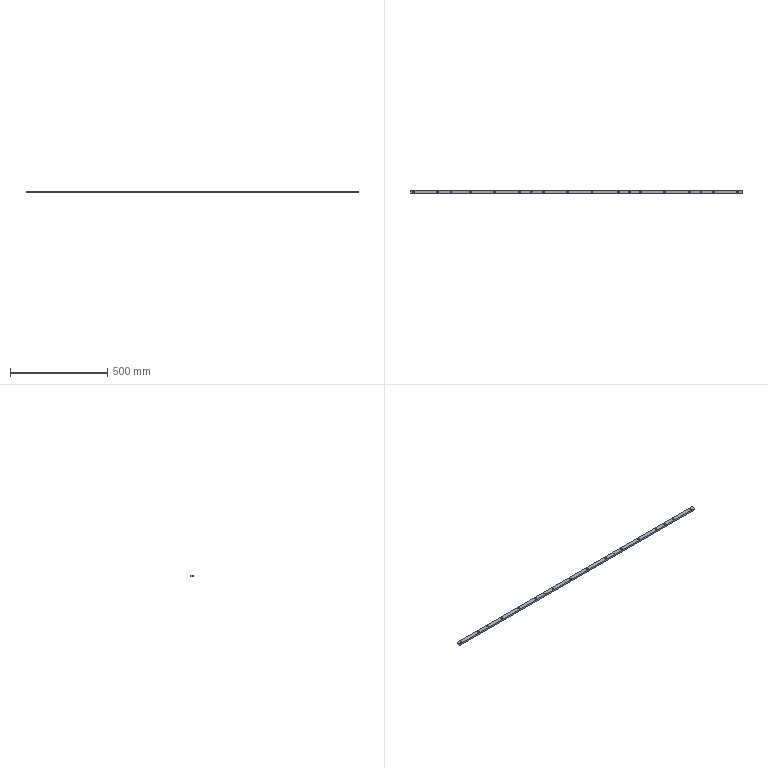Part | STEP file | J013-EBZ05-12-06-Part-1 | 1 solid | 46 faces | box 1710 x 19 x 9 mm | volume 281135 mm3 | cylinder 36 | plane 10 | commonest cylinder face diameters 10 x28 6.8 x8
STEP:
#1=CARTESIAN_POINT('',(1442.5,9.5,9.));
#2=VERTEX_POINT('',#1);
#3=CARTESIAN_POINT('',(1432.5,9.5,9.));
#4=VERTEX_POINT('',#3);
#5=CARTESIAN_POINT('',(1437.5,9.5,9.));
#6=DIRECTION('',(0.,0.,-1.));
#7=DIRECTION('',(-1.,0.,0.));
#8=AXIS2_PLACEMENT_3D('',#5,#6,#7);
#9=CIRCLE('',#8,5.);
#10=EDGE_CURVE('',#2,#4,#9,.T.);
#11=ORIENTED_EDGE('',*,*,#10,.F.);
#12=CARTESIAN_POINT('',(1442.5,9.5,0.));
#13=VERTEX_POINT('',#12);
#14=CARTESIAN_POINT('',(1442.5,9.5,9.));
#15=DIRECTION('',(0.,0.,-1.));
#16=VECTOR('',#15,1000.);
#17=LINE('',#14,#16);
#18=EDGE_CURVE('',#2,#13,#17,.T.);
#19=ORIENTED_EDGE('',*,*,#18,.T.);
#20=CARTESIAN_POINT('',(1432.5,9.5,0.));
#21=VERTEX_POINT('',#20);
#22=CARTESIAN_POINT('',(1437.5,9.5,0.));
#23=DIRECTION('',(0.,0.,1.));
#24=DIRECTION('',(1.,0.,0.));
#25=AXIS2_PLACEMENT_3D('',#22,#23,#24);
#26=CIRCLE('',#25,5.);
#27=EDGE_CURVE('',#21,#13,#26,.T.);
#28=ORIENTED_EDGE('',*,*,#27,.F.);
#29=CARTESIAN_POINT('',(1432.5,9.5,9.));
#30=DIRECTION('',(0.,0.,-1.));
#31=VECTOR('',#30,1000.);
#32=LINE('',#29,#31);
#33=EDGE_CURVE('',#4,#21,#32,.T.);
#34=ORIENTED_EDGE('',*,*,#33,.F.);
#35=EDGE_LOOP('',(#11,#19,#28,#34));
#36=FACE_OUTER_BOUND('',#35,.T.);
#37=CARTESIAN_POINT('',(1437.5,9.5,9.));
#38=DIRECTION('',(0.,0.,-1.));
#39=DIRECTION('',(-1.,0.,0.));
#40=AXIS2_PLACEMENT_3D('',#37,#38,#39);
#41=CYLINDRICAL_SURFACE('',#40,5.);
#42=ADVANCED_FACE('',(#36),#41,.F.);
#43=CARTESIAN_POINT('',(22.5,9.5,9.));
#44=VERTEX_POINT('',#43);
#45=CARTESIAN_POINT('',(12.5,9.5,9.));
#46=VERTEX_POINT('',#45);
#47=CARTESIAN_POINT('',(17.5,9.5,9.));
#48=DIRECTION('',(0.,0.,-1.));
#49=DIRECTION('',(-1.,0.,0.));
#50=AXIS2_PLACEMENT_3D('',#47,#48,#49);
#51=CIRCLE('',#50,5.);
#52=EDGE_CURVE('',#44,#46,#51,.T.);
#53=ORIENTED_EDGE('',*,*,#52,.F.);
#54=CARTESIAN_POINT('',(22.5,9.5,0.));
#55=VERTEX_POINT('',#54);
#56=CARTESIAN_POINT('',(22.5,9.5,9.));
#57=DIRECTION('',(0.,0.,-1.));
#58=VECTOR('',#57,1000.);
#59=LINE('',#56,#58);
#60=EDGE_CURVE('',#44,#55,#59,.T.);
#61=ORIENTED_EDGE('',*,*,#60,.T.);
#62=CARTESIAN_POINT('',(12.5,9.5,0.));
#63=VERTEX_POINT('',#62);
#64=CARTESIAN_POINT('',(17.5,9.5,0.));
#65=DIRECTION('',(0.,0.,1.));
#66=DIRECTION('',(1.,0.,0.));
#67=AXIS2_PLACEMENT_3D('',#64,#65,#66);
#68=CIRCLE('',#67,5.);
#69=EDGE_CURVE('',#63,#55,#68,.T.);
#70=ORIENTED_EDGE('',*,*,#69,.F.);
#71=CARTESIAN_POINT('',(12.5,9.5,9.));
#72=DIRECTION('',(0.,0.,-1.));
#73=VECTOR('',#72,1000.);
#74=LINE('',#71,#73);
#75=EDGE_CURVE('',#46,#63,#74,.T.);
#76=ORIENTED_EDGE('',*,*,#75,.F.);
#77=EDGE_LOOP('',(#53,#61,#70,#76));
#78=FACE_OUTER_BOUND('',#77,.T.);
#79=CARTESIAN_POINT('',(17.5,9.5,9.));
#80=DIRECTION('',(0.,0.,-1.));
#81=DIRECTION('',(-1.,0.,0.));
#82=AXIS2_PLACEMENT_3D('',#79,#80,#81);
#83=CYLINDRICAL_SURFACE('',#82,5.);
#84=ADVANCED_FACE('',(#78),#83,.F.);
#85=CARTESIAN_POINT('',(147.5,9.5,9.));
#86=VERTEX_POINT('',#85);
#87=CARTESIAN_POINT('',(137.5,9.5,9.));
#88=VERTEX_POINT('',#87);
#89=CARTESIAN_POINT('',(142.5,9.5,9.));
#90=DIRECTION('',(0.,0.,-1.));
#91=DIRECTION('',(-1.,0.,0.));
#92=AXIS2_PLACEMENT_3D('',#89,#90,#91);
#93=CIRCLE('',#92,5.);
#94=EDGE_CURVE('',#86,#88,#93,.T.);
#95=ORIENTED_EDGE('',*,*,#94,.F.);
#96=CARTESIAN_POINT('',(147.5,9.5,0.));
#97=VERTEX_POINT('',#96);
#98=CARTESIAN_POINT('',(147.5,9.5,9.));
#99=DIRECTION('',(0.,0.,-1.));
#100=VECTOR('',#99,1000.);
#101=LINE('',#98,#100);
#102=EDGE_CURVE('',#86,#97,#101,.T.);
#103=ORIENTED_EDGE('',*,*,#102,.T.);
#104=CARTESIAN_POINT('',(137.5,9.5,0.));
#105=VERTEX_POINT('',#104);
#106=CARTESIAN_POINT('',(142.5,9.5,0.));
#107=DIRECTION('',(0.,0.,1.));
#108=DIRECTION('',(1.,0.,0.));
#109=AXIS2_PLACEMENT_3D('',#106,#107,#108);
#110=CIRCLE('',#109,5.);
#111=EDGE_CURVE('',#105,#97,#110,.T.);
#112=ORIENTED_EDGE('',*,*,#111,.F.);
#113=CARTESIAN_POINT('',(137.5,9.5,9.));
#114=DIRECTION('',(0.,0.,-1.));
#115=VECTOR('',#114,1000.);
#116=LINE('',#113,#115);
#117=EDGE_CURVE('',#88,#105,#116,.T.);
#118=ORIENTED_EDGE('',*,*,#117,.F.);
#119=EDGE_LOOP('',(#95,#103,#112,#118));
#120=FACE_OUTER_BOUND('',#119,.T.);
#121=CARTESIAN_POINT('',(142.5,9.5,9.));
#122=DIRECTION('',(0.,0.,-1.));
#123=DIRECTION('',(-1.,0.,0.));
#124=AXIS2_PLACEMENT_3D('',#121,#122,#123);
#125=CYLINDRICAL_SURFACE('',#124,5.);
#126=ADVANCED_FACE('',(#120),#125,.F.);
#127=CARTESIAN_POINT('',(442.5,9.5,9.));
#128=VERTEX_POINT('',#127);
#129=CARTESIAN_POINT('',(432.5,9.5,9.));
#130=VERTEX_POINT('',#129);
#131=CARTESIAN_POINT('',(437.5,9.5,9.));
#132=DIRECTION('',(0.,0.,-1.));
#133=DIRECTION('',(-1.,0.,0.));
#134=AXIS2_PLACEMENT_3D('',#131,#132,#133);
#135=CIRCLE('',#134,5.);
#136=EDGE_CURVE('',#128,#130,#135,.T.);
#137=ORIENTED_EDGE('',*,*,#136,.F.);
#138=CARTESIAN_POINT('',(442.5,9.5,0.));
#139=VERTEX_POINT('',#138);
#140=CARTESIAN_POINT('',(442.5,9.5,9.));
#141=DIRECTION('',(0.,0.,-1.));
#142=VECTOR('',#141,1000.);
#143=LINE('',#140,#142);
#144=EDGE_CURVE('',#128,#139,#143,.T.);
#145=ORIENTED_EDGE('',*,*,#144,.T.);
#146=CARTESIAN_POINT('',(432.5,9.5,0.));
#147=VERTEX_POINT('',#146);
#148=CARTESIAN_POINT('',(437.5,9.5,0.));
#149=DIRECTION('',(0.,0.,1.));
#150=DIRECTION('',(1.,0.,0.));
#151=AXIS2_PLACEMENT_3D('',#148,#149,#150);
#152=CIRCLE('',#151,5.);
#153=EDGE_CURVE('',#147,#139,#152,.T.);
#154=ORIENTED_EDGE('',*,*,#153,.F.);
#155=CARTESIAN_POINT('',(432.5,9.5,9.));
#156=DIRECTION('',(0.,0.,-1.));
#157=VECTOR('',#156,1000.);
#158=LINE('',#155,#157);
#159=EDGE_CURVE('',#130,#147,#158,.T.);
#160=ORIENTED_EDGE('',*,*,#159,.F.);
#161=EDGE_LOOP('',(#137,#145,#154,#160));
#162=FACE_OUTER_BOUND('',#161,.T.);
#163=CARTESIAN_POINT('',(437.5,9.5,9.));
#164=DIRECTION('',(0.,0.,-1.));
#165=DIRECTION('',(-1.,0.,0.));
#166=AXIS2_PLACEMENT_3D('',#163,#164,#165);
#167=CYLINDRICAL_SURFACE('',#166,5.);
#168=ADVANCED_FACE('',(#162),#167,.F.);
#169=CARTESIAN_POINT('',(567.5,9.5,9.));
#170=VERTEX_POINT('',#169);
#171=CARTESIAN_POINT('',(557.5,9.5,9.));
#172=VERTEX_POINT('',#171);
#173=CARTESIAN_POINT('',(562.5,9.5,9.));
#174=DIRECTION('',(0.,0.,-1.));
#175=DIRECTION('',(-1.,0.,0.));
#176=AXIS2_PLACEMENT_3D('',#173,#174,#175);
#177=CIRCLE('',#176,5.);
#178=EDGE_CURVE('',#170,#172,#177,.T.);
#179=ORIENTED_EDGE('',*,*,#178,.F.);
#180=CARTESIAN_POINT('',(567.5,9.5,0.));
#181=VERTEX_POINT('',#180);
#182=CARTESIAN_POINT('',(567.5,9.5,9.));
#183=DIRECTION('',(0.,0.,-1.));
#184=VECTOR('',#183,1000.);
#185=LINE('',#182,#184);
#186=EDGE_CURVE('',#170,#181,#185,.T.);
#187=ORIENTED_EDGE('',*,*,#186,.T.);
#188=CARTESIAN_POINT('',(557.5,9.5,0.));
#189=VERTEX_POINT('',#188);
#190=CARTESIAN_POINT('',(562.5,9.5,0.));
#191=DIRECTION('',(0.,0.,1.));
#192=DIRECTION('',(1.,0.,0.));
#193=AXIS2_PLACEMENT_3D('',#190,#191,#192);
#194=CIRCLE('',#193,5.);
#195=EDGE_CURVE('',#189,#181,#194,.T.);
#196=ORIENTED_EDGE('',*,*,#195,.F.);
#197=CARTESIAN_POINT('',(557.5,9.5,9.));
#198=DIRECTION('',(0.,0.,-1.));
#199=VECTOR('',#198,1000.);
#200=LINE('',#197,#199);
#201=EDGE_CURVE('',#172,#189,#200,.T.);
#202=ORIENTED_EDGE('',*,*,#201,.F.);
#203=EDGE_LOOP('',(#179,#187,#196,#202));
#204=FACE_OUTER_BOUND('',#203,.T.);
#205=CARTESIAN_POINT('',(562.5,9.5,9.));
#206=DIRECTION('',(0.,0.,-1.));
#207=DIRECTION('',(-1.,0.,0.));
#208=AXIS2_PLACEMENT_3D('',#205,#206,#207);
#209=CYLINDRICAL_SURFACE('',#208,5.);
#210=ADVANCED_FACE('',(#204),#209,.F.);
#211=CARTESIAN_POINT('',(1692.5,9.5,9.));
#212=VERTEX_POINT('',#211);
#213=CARTESIAN_POINT('',(1682.5,9.5,9.));
#214=VERTEX_POINT('',#213);
#215=CARTESIAN_POINT('',(1687.5,9.5,9.));
#216=DIRECTION('',(0.,0.,-1.));
#217=DIRECTION('',(-1.,0.,0.));
#218=AXIS2_PLACEMENT_3D('',#215,#216,#217);
#219=CIRCLE('',#218,5.);
#220=EDGE_CURVE('',#212,#214,#219,.T.);
#221=ORIENTED_EDGE('',*,*,#220,.F.);
#222=CARTESIAN_POINT('',(1692.5,9.5,0.));
#223=VERTEX_POINT('',#222);
#224=CARTESIAN_POINT('',(1692.5,9.5,9.));
#225=DIRECTION('',(0.,0.,-1.));
#226=VECTOR('',#225,1000.);
#227=LINE('',#224,#226);
#228=EDGE_CURVE('',#212,#223,#227,.T.);
#229=ORIENTED_EDGE('',*,*,#228,.T.);
#230=CARTESIAN_POINT('',(1682.5,9.5,0.));
#231=VERTEX_POINT('',#230);
#232=CARTESIAN_POINT('',(1687.5,9.5,0.));
#233=DIRECTION('',(0.,0.,1.));
#234=DIRECTION('',(1.,0.,0.));
#235=AXIS2_PLACEMENT_3D('',#232,#233,#234);
#236=CIRCLE('',#235,5.);
#237=EDGE_CURVE('',#231,#223,#236,.T.);
#238=ORIENTED_EDGE('',*,*,#237,.F.);
#239=CARTESIAN_POINT('',(1682.5,9.5,9.));
#240=DIRECTION('',(0.,0.,-1.));
#241=VECTOR('',#240,1000.);
#242=LINE('',#239,#241);
#243=EDGE_CURVE('',#214,#231,#242,.T.);
#244=ORIENTED_EDGE('',*,*,#243,.F.);
#245=EDGE_LOOP('',(#221,#229,#238,#244));
#246=FACE_OUTER_BOUND('',#245,.T.);
#247=CARTESIAN_POINT('',(1687.5,9.5,9.));
#248=DIRECTION('',(0.,0.,-1.));
#249=DIRECTION('',(-1.,0.,0.));
#250=AXIS2_PLACEMENT_3D('',#247,#248,#249);
#251=CYLINDRICAL_SURFACE('',#250,5.);
#252=ADVANCED_FACE('',(#246),#251,.F.);
#253=CARTESIAN_POINT('',(1503.4,9.5,9.));
#254=VERTEX_POINT('',#253);
#255=CARTESIAN_POINT('',(1496.6,9.5,9.));
#256=VERTEX_POINT('',#255);
#257=CARTESIAN_POINT('',(1500.,9.5,9.));
#258=DIRECTION('',(0.,0.,-1.));
#259=DIRECTION('',(-1.,0.,0.));
#260=AXIS2_PLACEMENT_3D('',#257,#258,#259);
#261=CIRCLE('',#260,3.4);
#262=EDGE_CURVE('',#254,#256,#261,.T.);
#263=ORIENTED_EDGE('',*,*,#262,.F.);
#264=CARTESIAN_POINT('',(1503.4,9.5,0.));
#265=VERTEX_POINT('',#264);
#266=CARTESIAN_POINT('',(1503.4,9.5,9.));
#267=DIRECTION('',(0.,0.,-1.));
#268=VECTOR('',#267,1000.);
#269=LINE('',#266,#268);
#270=EDGE_CURVE('',#254,#265,#269,.T.);
#271=ORIENTED_EDGE('',*,*,#270,.T.);
#272=CARTESIAN_POINT('',(1496.6,9.5,0.));
#273=VERTEX_POINT('',#272);
#274=CARTESIAN_POINT('',(1500.,9.5,0.));
#275=DIRECTION('',(0.,0.,1.));
#276=DIRECTION('',(1.,0.,0.));
#277=AXIS2_PLACEMENT_3D('',#274,#275,#276);
#278=CIRCLE('',#277,3.4);
#279=EDGE_CURVE('',#273,#265,#278,.T.);
#280=ORIENTED_EDGE('',*,*,#279,.F.);
#281=CARTESIAN_POINT('',(1496.6,9.5,9.));
#282=DIRECTION('',(0.,0.,-1.));
#283=VECTOR('',#282,1000.);
#284=LINE('',#281,#283);
#285=EDGE_CURVE('',#256,#273,#284,.T.);
#286=ORIENTED_EDGE('',*,*,#285,.F.);
#287=EDGE_LOOP('',(#263,#271,#280,#286));
#288=FACE_OUTER_BOUND('',#287,.T.);
#289=CARTESIAN_POINT('',(1500.,9.5,9.));
#290=DIRECTION('',(0.,0.,-1.));
#291=DIRECTION('',(-1.,0.,0.));
#292=AXIS2_PLACEMENT_3D('',#289,#290,#291);
#293=CYLINDRICAL_SURFACE('',#292,3.4);
#294=ADVANCED_FACE('',(#288),#293,.F.);
#295=CARTESIAN_POINT('',(1133.4,9.5,9.));
#296=VERTEX_POINT('',#295);
#297=CARTESIAN_POINT('',(1126.6,9.5,9.));
#298=VERTEX_POINT('',#297);
#299=CARTESIAN_POINT('',(1130.,9.5,9.));
#300=DIRECTION('',(0.,0.,-1.));
#301=DIRECTION('',(-1.,0.,0.));
#302=AXIS2_PLACEMENT_3D('',#299,#300,#301);
#303=CIRCLE('',#302,3.4);
#304=EDGE_CURVE('',#296,#298,#303,.T.);
#305=ORIENTED_EDGE('',*,*,#304,.F.);
#306=CARTESIAN_POINT('',(1133.4,9.5,0.));
#307=VERTEX_POINT('',#306);
#308=CARTESIAN_POINT('',(1133.4,9.5,9.));
#309=DIRECTION('',(0.,0.,-1.));
#310=VECTOR('',#309,1000.);
#311=LINE('',#308,#310);
#312=EDGE_CURVE('',#296,#307,#311,.T.);
#313=ORIENTED_EDGE('',*,*,#312,.T.);
#314=CARTESIAN_POINT('',(1126.6,9.5,0.));
#315=VERTEX_POINT('',#314);
#316=CARTESIAN_POINT('',(1130.,9.5,0.));
#317=DIRECTION('',(0.,0.,1.));
#318=DIRECTION('',(1.,0.,0.));
#319=AXIS2_PLACEMENT_3D('',#316,#317,#318);
#320=CIRCLE('',#319,3.4);
#321=EDGE_CURVE('',#315,#307,#320,.T.);
#322=ORIENTED_EDGE('',*,*,#321,.F.);
#323=CARTESIAN_POINT('',(1126.6,9.5,9.));
#324=DIRECTION('',(0.,0.,-1.));
#325=VECTOR('',#324,1000.);
#326=LINE('',#323,#325);
#327=EDGE_CURVE('',#298,#315,#326,.T.);
#328=ORIENTED_EDGE('',*,*,#327,.F.);
#329=EDGE_LOOP('',(#305,#313,#322,#328));
#330=FACE_OUTER_BOUND('',#329,.T.);
#331=CARTESIAN_POINT('',(1130.,9.5,9.));
#332=DIRECTION('',(0.,0.,-1.));
#333=DIRECTION('',(-1.,0.,0.));
#334=AXIS2_PLACEMENT_3D('',#331,#332,#333);
#335=CYLINDRICAL_SURFACE('',#334,3.4);
#336=ADVANCED_FACE('',(#330),#335,.F.);
#337=CARTESIAN_POINT('',(628.4,9.5,9.));
#338=VERTEX_POINT('',#337);
#339=CARTESIAN_POINT('',(621.6,9.5,9.));
#340=VERTEX_POINT('',#339);
#341=CARTESIAN_POINT('',(625.,9.5,9.));
#342=DIRECTION('',(0.,0.,-1.));
#343=DIRECTION('',(-1.,0.,0.));
#344=AXIS2_PLACEMENT_3D('',#341,#342,#343);
#345=CIRCLE('',#344,3.4);
#346=EDGE_CURVE('',#338,#340,#345,.T.);
#347=ORIENTED_EDGE('',*,*,#346,.F.);
#348=CARTESIAN_POINT('',(628.4,9.5,0.));
#349=VERTEX_POINT('',#348);
#350=CARTESIAN_POINT('',(628.4,9.5,9.));
#351=DIRECTION('',(0.,0.,-1.));
#352=VECTOR('',#351,1000.);
#353=LINE('',#350,#352);
#354=EDGE_CURVE('',#338,#349,#353,.T.);
#355=ORIENTED_EDGE('',*,*,#354,.T.);
#356=CARTESIAN_POINT('',(621.6,9.5,0.));
#357=VERTEX_POINT('',#356);
#358=CARTESIAN_POINT('',(625.,9.5,0.));
#359=DIRECTION('',(0.,0.,1.));
#360=DIRECTION('',(1.,0.,0.));
#361=AXIS2_PLACEMENT_3D('',#358,#359,#360);
#362=CIRCLE('',#361,3.4);
#363=EDGE_CURVE('',#357,#349,#362,.T.);
#364=ORIENTED_EDGE('',*,*,#363,.F.);
#365=CARTESIAN_POINT('',(621.6,9.5,9.));
#366=DIRECTION('',(0.,0.,-1.));
#367=VECTOR('',#366,1000.);
#368=LINE('',#365,#367);
#369=EDGE_CURVE('',#340,#357,#368,.T.);
#370=ORIENTED_EDGE('',*,*,#369,.F.);
#371=EDGE_LOOP('',(#347,#355,#364,#370));
#372=FACE_OUTER_BOUND('',#371,.T.);
#373=CARTESIAN_POINT('',(625.,9.5,9.));
#374=DIRECTION('',(0.,0.,-1.));
#375=DIRECTION('',(-1.,0.,0.));
#376=AXIS2_PLACEMENT_3D('',#373,#374,#375);
#377=CYLINDRICAL_SURFACE('',#376,3.4);
#378=ADVANCED_FACE('',(#372),#377,.F.);
#379=CARTESIAN_POINT('',(213.9,9.5,9.));
#380=VERTEX_POINT('',#379);
#381=CARTESIAN_POINT('',(207.1,9.5,9.));
#382=VERTEX_POINT('',#381);
#383=CARTESIAN_POINT('',(210.5,9.5,9.));
#384=DIRECTION('',(0.,0.,-1.));
#385=DIRECTION('',(-1.,0.,0.));
#386=AXIS2_PLACEMENT_3D('',#383,#384,#385);
#387=CIRCLE('',#386,3.4);
#388=EDGE_CURVE('',#380,#382,#387,.T.);
#389=ORIENTED_EDGE('',*,*,#388,.F.);
#390=CARTESIAN_POINT('',(213.9,9.5,0.));
#391=VERTEX_POINT('',#390);
#392=CARTESIAN_POINT('',(213.9,9.5,9.));
#393=DIRECTION('',(0.,0.,-1.));
#394=VECTOR('',#393,1000.);
#395=LINE('',#392,#394);
#396=EDGE_CURVE('',#380,#391,#395,.T.);
#397=ORIENTED_EDGE('',*,*,#396,.T.);
#398=CARTESIAN_POINT('',(207.1,9.5,0.));
#399=VERTEX_POINT('',#398);
#400=CARTESIAN_POINT('',(210.5,9.5,0.));
#401=DIRECTION('',(0.,0.,1.));
#402=DIRECTION('',(1.,0.,0.));
#403=AXIS2_PLACEMENT_3D('',#400,#401,#402);
#404=CIRCLE('',#403,3.4);
#405=EDGE_CURVE('',#399,#391,#404,.T.);
#406=ORIENTED_EDGE('',*,*,#405,.F.);
#407=CARTESIAN_POINT('',(207.1,9.5,9.));
#408=DIRECTION('',(0.,0.,-1.));
#409=VECTOR('',#408,1000.);
#410=LINE('',#407,#409);
#411=EDGE_CURVE('',#382,#399,#410,.T.);
#412=ORIENTED_EDGE('',*,*,#411,.F.);
#413=EDGE_LOOP('',(#389,#397,#406,#412));
#414=FACE_OUTER_BOUND('',#413,.T.);
#415=CARTESIAN_POINT('',(210.5,9.5,9.));
#416=DIRECTION('',(0.,0.,-1.));
#417=DIRECTION('',(-1.,0.,0.));
#418=AXIS2_PLACEMENT_3D('',#415,#416,#417);
#419=CYLINDRICAL_SURFACE('',#418,3.4);
#420=ADVANCED_FACE('',(#414),#419,.F.);
#421=CARTESIAN_POINT('',(1077.5,9.5,9.));
#422=VERTEX_POINT('',#421);
#423=CARTESIAN_POINT('',(1067.5,9.5,9.));
#424=VERTEX_POINT('',#423);
#425=CARTESIAN_POINT('',(1072.5,9.5,9.));
#426=DIRECTION('',(0.,0.,-1.));
#427=DIRECTION('',(-1.,0.,0.));
#428=AXIS2_PLACEMENT_3D('',#425,#426,#427);
#429=CIRCLE('',#428,5.);
#430=EDGE_CURVE('',#422,#424,#429,.T.);
#431=ORIENTED_EDGE('',*,*,#430,.F.);
#432=CARTESIAN_POINT('',(1077.5,9.5,0.));
#433=VERTEX_POINT('',#432);
#434=CARTESIAN_POINT('',(1077.5,9.5,9.));
#435=DIRECTION('',(0.,0.,-1.));
#436=VECTOR('',#435,1000.);
#437=LINE('',#434,#436);
#438=EDGE_CURVE('',#422,#433,#437,.T.);
#439=ORIENTED_EDGE('',*,*,#438,.T.);
#440=CARTESIAN_POINT('',(1067.5,9.5,0.));
#441=VERTEX_POINT('',#440);
#442=CARTESIAN_POINT('',(1072.5,9.5,0.));
#443=DIRECTION('',(0.,0.,1.));
#444=DIRECTION('',(1.,0.,0.));
#445=AXIS2_PLACEMENT_3D('',#442,#443,#444);
#446=CIRCLE('',#445,5.);
#447=EDGE_CURVE('',#441,#433,#446,.T.);
#448=ORIENTED_EDGE('',*,*,#447,.F.);
#449=CARTESIAN_POINT('',(1067.5,9.5,9.));
#450=DIRECTION('',(0.,0.,-1.));
#451=VECTOR('',#450,1000.);
#452=LINE('',#449,#451);
#453=EDGE_CURVE('',#424,#441,#452,.T.);
#454=ORIENTED_EDGE('',*,*,#453,.F.);
#455=EDGE_LOOP('',(#431,#439,#448,#454));
#456=FACE_OUTER_BOUND('',#455,.T.);
#457=CARTESIAN_POINT('',(1072.5,9.5,9.));
#458=DIRECTION('',(0.,0.,-1.));
#459=DIRECTION('',(-1.,0.,0.));
#460=AXIS2_PLACEMENT_3D('',#457,#458,#459);
#461=CYLINDRICAL_SURFACE('',#460,5.);
#462=ADVANCED_FACE('',(#456),#461,.F.);
#463=CARTESIAN_POINT('',(1192.5,9.5,9.));
#464=VERTEX_POINT('',#463);
#465=CARTESIAN_POINT('',(1182.5,9.5,9.));
#466=VERTEX_POINT('',#465);
#467=CARTESIAN_POINT('',(1187.5,9.5,9.));
#468=DIRECTION('',(0.,0.,-1.));
#469=DIRECTION('',(-1.,0.,0.));
#470=AXIS2_PLACEMENT_3D('',#467,#468,#469);
#471=CIRCLE('',#470,5.);
#472=EDGE_CURVE('',#464,#466,#471,.T.);
#473=ORIENTED_EDGE('',*,*,#472,.F.);
#474=CARTESIAN_POINT('',(1192.5,9.5,0.));
#475=VERTEX_POINT('',#474);
#476=CARTESIAN_POINT('',(1192.5,9.5,9.));
#477=DIRECTION('',(0.,0.,-1.));
#478=VECTOR('',#477,1000.);
#479=LINE('',#476,#478);
#480=EDGE_CURVE('',#464,#475,#479,.T.);
#481=ORIENTED_EDGE('',*,*,#480,.T.);
#482=CARTESIAN_POINT('',(1182.5,9.5,0.));
#483=VERTEX_POINT('',#482);
#484=CARTESIAN_POINT('',(1187.5,9.5,0.));
#485=DIRECTION('',(0.,0.,1.));
#486=DIRECTION('',(1.,0.,0.));
#487=AXIS2_PLACEMENT_3D('',#484,#485,#486);
#488=CIRCLE('',#487,5.);
#489=EDGE_CURVE('',#483,#475,#488,.T.);
#490=ORIENTED_EDGE('',*,*,#489,.F.);
#491=CARTESIAN_POINT('',(1182.5,9.5,9.));
#492=DIRECTION('',(0.,0.,-1.));
#493=VECTOR('',#492,1000.);
#494=LINE('',#491,#493);
#495=EDGE_CURVE('',#466,#483,#494,.T.);
#496=ORIENTED_EDGE('',*,*,#495,.F.);
#497=EDGE_LOOP('',(#473,#481,#490,#496));
#498=FACE_OUTER_BOUND('',#497,.T.);
#499=CARTESIAN_POINT('',(1187.5,9.5,9.));
#500=DIRECTION('',(0.,0.,-1.));
#501=DIRECTION('',(-1.,0.,0.));
#502=AXIS2_PLACEMENT_3D('',#499,#500,#501);
#503=CYLINDRICAL_SURFACE('',#502,5.);
#504=ADVANCED_FACE('',(#498),#503,.F.);
#505=CARTESIAN_POINT('',(1317.5,9.5,9.));
#506=VERTEX_POINT('',#505);
#507=CARTESIAN_POINT('',(1307.5,9.5,9.));
#508=VERTEX_POINT('',#507);
#509=CARTESIAN_POINT('',(1312.5,9.5,9.));
#510=DIRECTION('',(0.,0.,-1.));
#511=DIRECTION('',(-1.,0.,0.));
#512=AXIS2_PLACEMENT_3D('',#509,#510,#511);
#513=CIRCLE('',#512,5.);
#514=EDGE_CURVE('',#506,#508,#513,.T.);
#515=ORIENTED_EDGE('',*,*,#514,.F.);
#516=CARTESIAN_POINT('',(1317.5,9.5,0.));
#517=VERTEX_POINT('',#516);
#518=CARTESIAN_POINT('',(1317.5,9.5,9.));
#519=DIRECTION('',(0.,0.,-1.));
#520=VECTOR('',#519,1000.);
#521=LINE('',#518,#520);
#522=EDGE_CURVE('',#506,#517,#521,.T.);
#523=ORIENTED_EDGE('',*,*,#522,.T.);
#524=CARTESIAN_POINT('',(1307.5,9.5,0.));
#525=VERTEX_POINT('',#524);
#526=CARTESIAN_POINT('',(1312.5,9.5,0.));
#527=DIRECTION('',(0.,0.,1.));
#528=DIRECTION('',(1.,0.,0.));
#529=AXIS2_PLACEMENT_3D('',#526,#527,#528);
#530=CIRCLE('',#529,5.);
#531=EDGE_CURVE('',#525,#517,#530,.T.);
#532=ORIENTED_EDGE('',*,*,#531,.F.);
#533=CARTESIAN_POINT('',(1307.5,9.5,9.));
#534=DIRECTION('',(0.,0.,-1.));
#535=VECTOR('',#534,1000.);
#536=LINE('',#533,#535);
#537=EDGE_CURVE('',#508,#525,#536,.T.);
#538=ORIENTED_EDGE('',*,*,#537,.F.);
#539=EDGE_LOOP('',(#515,#523,#532,#538));
#540=FACE_OUTER_BOUND('',#539,.T.);
#541=CARTESIAN_POINT('',(1312.5,9.5,9.));
#542=DIRECTION('',(0.,0.,-1.));
#543=DIRECTION('',(-1.,0.,0.));
#544=AXIS2_PLACEMENT_3D('',#541,#542,#543);
#545=CYLINDRICAL_SURFACE('',#544,5.);
#546=ADVANCED_FACE('',(#540),#545,.F.);
#547=CARTESIAN_POINT('',(317.5,9.5,9.));
#548=VERTEX_POINT('',#547);
#549=CARTESIAN_POINT('',(307.5,9.5,9.));
#550=VERTEX_POINT('',#549);
#551=CARTESIAN_POINT('',(312.5,9.5,9.));
#552=DIRECTION('',(0.,0.,-1.));
#553=DIRECTION('',(-1.,0.,0.));
#554=AXIS2_PLACEMENT_3D('',#551,#552,#553);
#555=CIRCLE('',#554,5.);
#556=EDGE_CURVE('',#548,#550,#555,.T.);
#557=ORIENTED_EDGE('',*,*,#556,.F.);
#558=CARTESIAN_POINT('',(317.5,9.5,0.));
#559=VERTEX_POINT('',#558);
#560=CARTESIAN_POINT('',(317.5,9.5,9.));
#561=DIRECTION('',(0.,0.,-1.));
#562=VECTOR('',#561,1000.);
#563=LINE('',#560,#562);
#564=EDGE_CURVE('',#548,#559,#563,.T.);
#565=ORIENTED_EDGE('',*,*,#564,.T.);
#566=CARTESIAN_POINT('',(307.5,9.5,0.));
#567=VERTEX_POINT('',#566);
#568=CARTESIAN_POINT('',(312.5,9.5,0.));
#569=DIRECTION('',(0.,0.,1.));
#570=DIRECTION('',(1.,0.,0.));
#571=AXIS2_PLACEMENT_3D('',#568,#569,#570);
#572=CIRCLE('',#571,5.);
#573=EDGE_CURVE('',#567,#559,#572,.T.);
#574=ORIENTED_EDGE('',*,*,#573,.F.);
#575=CARTESIAN_POINT('',(307.5,9.5,9.));
#576=DIRECTION('',(0.,0.,-1.));
#577=VECTOR('',#576,1000.);
#578=LINE('',#575,#577);
#579=EDGE_CURVE('',#550,#567,#578,.T.);
#580=ORIENTED_EDGE('',*,*,#579,.F.);
#581=EDGE_LOOP('',(#557,#565,#574,#580));
#582=FACE_OUTER_BOUND('',#581,.T.);
#583=CARTESIAN_POINT('',(312.5,9.5,9.));
#584=DIRECTION('',(0.,0.,-1.));
#585=DIRECTION('',(-1.,0.,0.));
#586=AXIS2_PLACEMENT_3D('',#583,#584,#585);
#587=CYLINDRICAL_SURFACE('',#586,5.);
#588=ADVANCED_FACE('',(#582),#587,.F.);
#589=CARTESIAN_POINT('',(692.5,9.5,9.));
#590=VERTEX_POINT('',#589);
#591=CARTESIAN_POINT('',(682.5,9.5,9.));
#592=VERTEX_POINT('',#591);
#593=CARTESIAN_POINT('',(687.5,9.5,9.));
#594=DIRECTION('',(0.,0.,-1.));
#595=DIRECTION('',(-1.,0.,0.));
#596=AXIS2_PLACEMENT_3D('',#593,#594,#595);
#597=CIRCLE('',#596,5.);
#598=EDGE_CURVE('',#590,#592,#597,.T.);
#599=ORIENTED_EDGE('',*,*,#598,.F.);
#600=CARTESIAN_POINT('',(692.5,9.5,0.));
#601=VERTEX_POINT('',#600);
#602=CARTESIAN_POINT('',(692.5,9.5,9.));
#603=DIRECTION('',(0.,0.,-1.));
#604=VECTOR('',#603,1000.);
#605=LINE('',#602,#604);
#606=EDGE_CURVE('',#590,#601,#605,.T.);
#607=ORIENTED_EDGE('',*,*,#606,.T.);
#608=CARTESIAN_POINT('',(682.5,9.5,0.));
#609=VERTEX_POINT('',#608);
#610=CARTESIAN_POINT('',(687.5,9.5,0.));
#611=DIRECTION('',(0.,0.,1.));
#612=DIRECTION('',(1.,0.,0.));
#613=AXIS2_PLACEMENT_3D('',#610,#611,#612);
#614=CIRCLE('',#613,5.);
#615=EDGE_CURVE('',#609,#601,#614,.T.);
#616=ORIENTED_EDGE('',*,*,#615,.F.);
#617=CARTESIAN_POINT('',(682.5,9.5,9.));
#618=DIRECTION('',(0.,0.,-1.));
#619=VECTOR('',#618,1000.);
#620=LINE('',#617,#619);
#621=EDGE_CURVE('',#592,#609,#620,.T.);
#622=ORIENTED_EDGE('',*,*,#621,.F.);
#623=EDGE_LOOP('',(#599,#607,#616,#622));
#624=FACE_OUTER_BOUND('',#623,.T.);
#625=CARTESIAN_POINT('',(687.5,9.5,9.));
#626=DIRECTION('',(0.,0.,-1.));
#627=DIRECTION('',(-1.,0.,0.));
#628=AXIS2_PLACEMENT_3D('',#625,#626,#627);
#629=CYLINDRICAL_SURFACE('',#628,5.);
#630=ADVANCED_FACE('',(#624),#629,.F.);
#631=CARTESIAN_POINT('',(817.5,9.5,9.));
#632=VERTEX_POINT('',#631);
#633=CARTESIAN_POINT('',(807.5,9.5,9.));
#634=VERTEX_POINT('',#633);
#635=CARTESIAN_POINT('',(812.5,9.5,9.));
#636=DIRECTION('',(0.,0.,-1.));
#637=DIRECTION('',(-1.,0.,0.));
#638=AXIS2_PLACEMENT_3D('',#635,#636,#637);
#639=CIRCLE('',#638,5.);
#640=EDGE_CURVE('',#632,#634,#639,.T.);
#641=ORIENTED_EDGE('',*,*,#640,.F.);
#642=CARTESIAN_POINT('',(817.5,9.5,0.));
#643=VERTEX_POINT('',#642);
#644=CARTESIAN_POINT('',(817.5,9.5,9.));
#645=DIRECTION('',(0.,0.,-1.));
#646=VECTOR('',#645,1000.);
#647=LINE('',#644,#646);
#648=EDGE_CURVE('',#632,#643,#647,.T.);
#649=ORIENTED_EDGE('',*,*,#648,.T.);
#650=CARTESIAN_POINT('',(807.5,9.5,0.));
#651=VERTEX_POINT('',#650);
#652=CARTESIAN_POINT('',(812.5,9.5,0.));
#653=DIRECTION('',(0.,0.,1.));
#654=DIRECTION('',(1.,0.,0.));
#655=AXIS2_PLACEMENT_3D('',#652,#653,#654);
#656=CIRCLE('',#655,5.);
#657=EDGE_CURVE('',#651,#643,#656,.T.);
#658=ORIENTED_EDGE('',*,*,#657,.F.);
#659=CARTESIAN_POINT('',(807.5,9.5,9.));
#660=DIRECTION('',(0.,0.,-1.));
#661=VECTOR('',#660,1000.);
#662=LINE('',#659,#661);
#663=EDGE_CURVE('',#634,#651,#662,.T.);
#664=ORIENTED_EDGE('',*,*,#663,.F.);
#665=EDGE_LOOP('',(#641,#649,#658,#664));
#666=FACE_OUTER_BOUND('',#665,.T.);
#667=CARTESIAN_POINT('',(812.5,9.5,9.));
#668=DIRECTION('',(0.,0.,-1.));
#669=DIRECTION('',(-1.,0.,0.));
#670=AXIS2_PLACEMENT_3D('',#667,#668,#669);
#671=CYLINDRICAL_SURFACE('',#670,5.);
#672=ADVANCED_FACE('',(#666),#671,.F.);
#673=CARTESIAN_POINT('',(942.5,9.5,9.));
#674=VERTEX_POINT('',#673);
#675=CARTESIAN_POINT('',(932.5,9.5,9.));
#676=VERTEX_POINT('',#675);
#677=CARTESIAN_POINT('',(937.5,9.5,9.));
#678=DIRECTION('',(0.,0.,-1.));
#679=DIRECTION('',(-1.,0.,0.));
#680=AXIS2_PLACEMENT_3D('',#677,#678,#679);
#681=CIRCLE('',#680,5.);
#682=EDGE_CURVE('',#674,#676,#681,.T.);
#683=ORIENTED_EDGE('',*,*,#682,.F.);
#684=CARTESIAN_POINT('',(942.5,9.5,0.));
#685=VERTEX_POINT('',#684);
#686=CARTESIAN_POINT('',(942.5,9.5,9.));
#687=DIRECTION('',(0.,0.,-1.));
#688=VECTOR('',#687,1000.);
#689=LINE('',#686,#688);
#690=EDGE_CURVE('',#674,#685,#689,.T.);
#691=ORIENTED_EDGE('',*,*,#690,.T.);
#692=CARTESIAN_POINT('',(932.5,9.5,0.));
#693=VERTEX_POINT('',#692);
#694=CARTESIAN_POINT('',(937.5,9.5,0.));
#695=DIRECTION('',(0.,0.,1.));
#696=DIRECTION('',(1.,0.,0.));
#697=AXIS2_PLACEMENT_3D('',#694,#695,#696);
#698=CIRCLE('',#697,5.);
#699=EDGE_CURVE('',#693,#685,#698,.T.);
#700=ORIENTED_EDGE('',*,*,#699,.F.);
#701=CARTESIAN_POINT('',(932.5,9.5,9.));
#702=DIRECTION('',(0.,0.,-1.));
#703=VECTOR('',#702,1000.);
#704=LINE('',#701,#703);
#705=EDGE_CURVE('',#676,#693,#704,.T.);
#706=ORIENTED_EDGE('',*,*,#705,.F.);
#707=EDGE_LOOP('',(#683,#691,#700,#706));
#708=FACE_OUTER_BOUND('',#707,.T.);
#709=CARTESIAN_POINT('',(937.5,9.5,9.));
#710=DIRECTION('',(0.,0.,-1.));
#711=DIRECTION('',(-1.,0.,0.));
#712=AXIS2_PLACEMENT_3D('',#709,#710,#711);
#713=CYLINDRICAL_SURFACE('',#712,5.);
#714=ADVANCED_FACE('',(#708),#713,.F.);
#715=CARTESIAN_POINT('',(1567.5,9.5,9.));
#716=VERTEX_POINT('',#715);
#717=CARTESIAN_POINT('',(1557.5,9.5,9.));
#718=VERTEX_POINT('',#717);
#719=CARTESIAN_POINT('',(1562.5,9.5,9.));
#720=DIRECTION('',(0.,0.,-1.));
#721=DIRECTION('',(-1.,0.,0.));
#722=AXIS2_PLACEMENT_3D('',#719,#720,#721);
#723=CIRCLE('',#722,5.);
#724=EDGE_CURVE('',#716,#718,#723,.T.);
#725=ORIENTED_EDGE('',*,*,#724,.F.);
#726=CARTESIAN_POINT('',(1567.5,9.5,0.));
#727=VERTEX_POINT('',#726);
#728=CARTESIAN_POINT('',(1567.5,9.5,9.));
#729=DIRECTION('',(0.,0.,-1.));
#730=VECTOR('',#729,1000.);
#731=LINE('',#728,#730);
#732=EDGE_CURVE('',#716,#727,#731,.T.);
#733=ORIENTED_EDGE('',*,*,#732,.T.);
#734=CARTESIAN_POINT('',(1557.5,9.5,0.));
#735=VERTEX_POINT('',#734);
#736=CARTESIAN_POINT('',(1562.5,9.5,0.));
#737=DIRECTION('',(0.,0.,1.));
#738=DIRECTION('',(1.,0.,0.));
#739=AXIS2_PLACEMENT_3D('',#736,#737,#738);
#740=CIRCLE('',#739,5.);
#741=EDGE_CURVE('',#735,#727,#740,.T.);
#742=ORIENTED_EDGE('',*,*,#741,.F.);
#743=CARTESIAN_POINT('',(1557.5,9.5,9.));
#744=DIRECTION('',(0.,0.,-1.));
#745=VECTOR('',#744,1000.);
#746=LINE('',#743,#745);
#747=EDGE_CURVE('',#718,#735,#746,.T.);
#748=ORIENTED_EDGE('',*,*,#747,.F.);
#749=EDGE_LOOP('',(#725,#733,#742,#748));
#750=FACE_OUTER_BOUND('',#749,.T.);
#751=CARTESIAN_POINT('',(1562.5,9.5,9.));
#752=DIRECTION('',(0.,0.,-1.));
#753=DIRECTION('',(-1.,0.,0.));
#754=AXIS2_PLACEMENT_3D('',#751,#752,#753);
#755=CYLINDRICAL_SURFACE('',#754,5.);
#756=ADVANCED_FACE('',(#750),#755,.F.);
#757=CARTESIAN_POINT('',(1437.5,9.5,9.));
#758=DIRECTION('',(0.,0.,-1.));
#759=DIRECTION('',(-1.,0.,0.));
#760=AXIS2_PLACEMENT_3D('',#757,#758,#759);
#761=CIRCLE('',#760,5.);
#762=EDGE_CURVE('',#4,#2,#761,.T.);
#763=ORIENTED_EDGE('',*,*,#762,.T.);
#764=ORIENTED_EDGE('',*,*,#10,.T.);
#765=EDGE_LOOP('',(#763,#764));
#766=FACE_BOUND('',#765,.T.);
#767=CARTESIAN_POINT('',(17.5,9.5,9.));
#768=DIRECTION('',(0.,0.,-1.));
#769=DIRECTION('',(-1.,0.,0.));
#770=AXIS2_PLACEMENT_3D('',#767,#768,#769);
#771=CIRCLE('',#770,5.);
#772=EDGE_CURVE('',#46,#44,#771,.T.);
#773=ORIENTED_EDGE('',*,*,#772,.T.);
#774=ORIENTED_EDGE('',*,*,#52,.T.);
#775=EDGE_LOOP('',(#773,#774));
#776=FACE_BOUND('',#775,.T.);
#777=CARTESIAN_POINT('',(142.5,9.5,9.));
#778=DIRECTION('',(0.,0.,-1.));
#779=DIRECTION('',(-1.,0.,0.));
#780=AXIS2_PLACEMENT_3D('',#777,#778,#779);
#781=CIRCLE('',#780,5.);
#782=EDGE_CURVE('',#88,#86,#781,.T.);
#783=ORIENTED_EDGE('',*,*,#782,.T.);
#784=ORIENTED_EDGE('',*,*,#94,.T.);
#785=EDGE_LOOP('',(#783,#784));
#786=FACE_BOUND('',#785,.T.);
#787=CARTESIAN_POINT('',(437.5,9.5,9.));
#788=DIRECTION('',(0.,0.,-1.));
#789=DIRECTION('',(-1.,0.,0.));
#790=AXIS2_PLACEMENT_3D('',#787,#788,#789);
#791=CIRCLE('',#790,5.);
#792=EDGE_CURVE('',#130,#128,#791,.T.);
#793=ORIENTED_EDGE('',*,*,#792,.T.);
#794=ORIENTED_EDGE('',*,*,#136,.T.);
#795=EDGE_LOOP('',(#793,#794));
#796=FACE_BOUND('',#795,.T.);
#797=CARTESIAN_POINT('',(562.5,9.5,9.));
#798=DIRECTION('',(0.,0.,-1.));
#799=DIRECTION('',(-1.,0.,0.));
#800=AXIS2_PLACEMENT_3D('',#797,#798,#799);
#801=CIRCLE('',#800,5.);
#802=EDGE_CURVE('',#172,#170,#801,.T.);
#803=ORIENTED_EDGE('',*,*,#802,.T.);
#804=ORIENTED_EDGE('',*,*,#178,.T.);
#805=EDGE_LOOP('',(#803,#804));
#806=FACE_BOUND('',#805,.T.);
#807=CARTESIAN_POINT('',(1687.5,9.5,9.));
#808=DIRECTION('',(0.,0.,-1.));
#809=DIRECTION('',(-1.,0.,0.));
#810=AXIS2_PLACEMENT_3D('',#807,#808,#809);
#811=CIRCLE('',#810,5.);
#812=EDGE_CURVE('',#214,#212,#811,.T.);
#813=ORIENTED_EDGE('',*,*,#812,.T.);
#814=ORIENTED_EDGE('',*,*,#220,.T.);
#815=EDGE_LOOP('',(#813,#814));
#816=FACE_BOUND('',#815,.T.);
#817=CARTESIAN_POINT('',(1500.,9.5,9.));
#818=DIRECTION('',(0.,0.,-1.));
#819=DIRECTION('',(-1.,0.,0.));
#820=AXIS2_PLACEMENT_3D('',#817,#818,#819);
#821=CIRCLE('',#820,3.4);
#822=EDGE_CURVE('',#256,#254,#821,.T.);
#823=ORIENTED_EDGE('',*,*,#822,.T.);
#824=ORIENTED_EDGE('',*,*,#262,.T.);
#825=EDGE_LOOP('',(#823,#824));
#826=FACE_BOUND('',#825,.T.);
#827=CARTESIAN_POINT('',(1130.,9.5,9.));
#828=DIRECTION('',(0.,0.,-1.));
#829=DIRECTION('',(-1.,0.,0.));
#830=AXIS2_PLACEMENT_3D('',#827,#828,#829);
#831=CIRCLE('',#830,3.4);
#832=EDGE_CURVE('',#298,#296,#831,.T.);
#833=ORIENTED_EDGE('',*,*,#832,.T.);
#834=ORIENTED_EDGE('',*,*,#304,.T.);
#835=EDGE_LOOP('',(#833,#834));
#836=FACE_BOUND('',#835,.T.);
#837=CARTESIAN_POINT('',(625.,9.5,9.));
#838=DIRECTION('',(0.,0.,-1.));
#839=DIRECTION('',(-1.,0.,0.));
#840=AXIS2_PLACEMENT_3D('',#837,#838,#839);
#841=CIRCLE('',#840,3.4);
#842=EDGE_CURVE('',#340,#338,#841,.T.);
#843=ORIENTED_EDGE('',*,*,#842,.T.);
#844=ORIENTED_EDGE('',*,*,#346,.T.);
#845=EDGE_LOOP('',(#843,#844));
#846=FACE_BOUND('',#845,.T.);
#847=CARTESIAN_POINT('',(210.5,9.5,9.));
#848=DIRECTION('',(0.,0.,-1.));
#849=DIRECTION('',(-1.,0.,0.));
#850=AXIS2_PLACEMENT_3D('',#847,#848,#849);
#851=CIRCLE('',#850,3.4);
#852=EDGE_CURVE('',#382,#380,#851,.T.);
#853=ORIENTED_EDGE('',*,*,#852,.T.);
#854=ORIENTED_EDGE('',*,*,#388,.T.);
#855=EDGE_LOOP('',(#853,#854));
#856=FACE_BOUND('',#855,.T.);
#857=CARTESIAN_POINT('',(1072.5,9.5,9.));
#858=DIRECTION('',(0.,0.,-1.));
#859=DIRECTION('',(-1.,0.,0.));
#860=AXIS2_PLACEMENT_3D('',#857,#858,#859);
#861=CIRCLE('',#860,5.);
#862=EDGE_CURVE('',#424,#422,#861,.T.);
#863=ORIENTED_EDGE('',*,*,#862,.T.);
#864=ORIENTED_EDGE('',*,*,#430,.T.);
#865=EDGE_LOOP('',(#863,#864));
#866=FACE_BOUND('',#865,.T.);
#867=CARTESIAN_POINT('',(1187.5,9.5,9.));
#868=DIRECTION('',(0.,0.,-1.));
#869=DIRECTION('',(-1.,0.,0.));
#870=AXIS2_PLACEMENT_3D('',#867,#868,#869);
#871=CIRCLE('',#870,5.);
#872=EDGE_CURVE('',#466,#464,#871,.T.);
#873=ORIENTED_EDGE('',*,*,#872,.T.);
#874=ORIENTED_EDGE('',*,*,#472,.T.);
#875=EDGE_LOOP('',(#873,#874));
#876=FACE_BOUND('',#875,.T.);
#877=CARTESIAN_POINT('',(1312.5,9.5,9.));
#878=DIRECTION('',(0.,0.,-1.));
#879=DIRECTION('',(-1.,0.,0.));
#880=AXIS2_PLACEMENT_3D('',#877,#878,#879);
#881=CIRCLE('',#880,5.);
#882=EDGE_CURVE('',#508,#506,#881,.T.);
#883=ORIENTED_EDGE('',*,*,#882,.T.);
#884=ORIENTED_EDGE('',*,*,#514,.T.);
#885=EDGE_LOOP('',(#883,#884));
#886=FACE_BOUND('',#885,.T.);
#887=CARTESIAN_POINT('',(312.5,9.5,9.));
#888=DIRECTION('',(0.,0.,-1.));
#889=DIRECTION('',(-1.,0.,0.));
#890=AXIS2_PLACEMENT_3D('',#887,#888,#889);
#891=CIRCLE('',#890,5.);
#892=EDGE_CURVE('',#550,#548,#891,.T.);
#893=ORIENTED_EDGE('',*,*,#892,.T.);
#894=ORIENTED_EDGE('',*,*,#556,.T.);
#895=EDGE_LOOP('',(#893,#894));
#896=FACE_BOUND('',#895,.T.);
#897=CARTESIAN_POINT('',(687.5,9.5,9.));
#898=DIRECTION('',(0.,0.,-1.));
#899=DIRECTION('',(-1.,0.,0.));
#900=AXIS2_PLACEMENT_3D('',#897,#898,#899);
#901=CIRCLE('',#900,5.);
#902=EDGE_CURVE('',#592,#590,#901,.T.);
#903=ORIENTED_EDGE('',*,*,#902,.T.);
#904=ORIENTED_EDGE('',*,*,#598,.T.);
#905=EDGE_LOOP('',(#903,#904));
#906=FACE_BOUND('',#905,.T.);
#907=CARTESIAN_POINT('',(812.5,9.5,9.));
#908=DIRECTION('',(0.,0.,-1.));
#909=DIRECTION('',(-1.,0.,0.));
#910=AXIS2_PLACEMENT_3D('',#907,#908,#909);
#911=CIRCLE('',#910,5.);
#912=EDGE_CURVE('',#634,#632,#911,.T.);
#913=ORIENTED_EDGE('',*,*,#912,.T.);
#914=ORIENTED_EDGE('',*,*,#640,.T.);
#915=EDGE_LOOP('',(#913,#914));
#916=FACE_BOUND('',#915,.T.);
#917=CARTESIAN_POINT('',(937.5,9.5,9.));
#918=DIRECTION('',(0.,0.,-1.));
#919=DIRECTION('',(-1.,0.,0.));
#920=AXIS2_PLACEMENT_3D('',#917,#918,#919);
#921=CIRCLE('',#920,5.);
#922=EDGE_CURVE('',#676,#674,#921,.T.);
#923=ORIENTED_EDGE('',*,*,#922,.T.);
#924=ORIENTED_EDGE('',*,*,#682,.T.);
#925=EDGE_LOOP('',(#923,#924));
#926=FACE_BOUND('',#925,.T.);
#927=CARTESIAN_POINT('',(1562.5,9.5,9.));
#928=DIRECTION('',(0.,0.,-1.));
#929=DIRECTION('',(-1.,0.,0.));
#930=AXIS2_PLACEMENT_3D('',#927,#928,#929);
#931=CIRCLE('',#930,5.);
#932=EDGE_CURVE('',#718,#716,#931,.T.);
#933=ORIENTED_EDGE('',*,*,#932,.T.);
#934=ORIENTED_EDGE('',*,*,#724,.T.);
#935=EDGE_LOOP('',(#933,#934));
#936=FACE_BOUND('',#935,.T.);
#937=CARTESIAN_POINT('',(1708.,0.,9.));
#938=VERTEX_POINT('',#937);
#939=CARTESIAN_POINT('',(2.,0.,9.));
#940=VERTEX_POINT('',#939);
#941=CARTESIAN_POINT('',(855.,0.,9.));
#942=DIRECTION('',(-1.,0.,0.));
#943=VECTOR('',#942,1000.);
#944=LINE('',#941,#943);
#945=EDGE_CURVE('',#938,#940,#944,.T.);
#946=ORIENTED_EDGE('',*,*,#945,.F.);
#947=CARTESIAN_POINT('',(1710.,2.,9.));
#948=VERTEX_POINT('',#947);
#949=CARTESIAN_POINT('',(1286.25,-421.75,9.));
#950=DIRECTION('',(0.7071,0.7071,0.));
#951=VECTOR('',#950,1000.);
#952=LINE('',#949,#951);
#953=EDGE_CURVE('',#938,#948,#952,.T.);
#954=ORIENTED_EDGE('',*,*,#953,.T.);
#955=CARTESIAN_POINT('',(1710.,17.,9.));
#956=VERTEX_POINT('',#955);
#957=CARTESIAN_POINT('',(1710.,9.5,9.));
#958=DIRECTION('',(0.,-1.,0.));
#959=VECTOR('',#958,1000.);
#960=LINE('',#957,#959);
#961=EDGE_CURVE('',#956,#948,#960,.T.);
#962=ORIENTED_EDGE('',*,*,#961,.F.);
#963=CARTESIAN_POINT('',(1708.,19.,9.));
#964=VERTEX_POINT('',#963);
#965=CARTESIAN_POINT('',(1286.25,440.75,9.));
#966=DIRECTION('',(-0.7071,0.7071,0.));
#967=VECTOR('',#966,1000.);
#968=LINE('',#965,#967);
#969=EDGE_CURVE('',#956,#964,#968,.T.);
#970=ORIENTED_EDGE('',*,*,#969,.T.);
#971=CARTESIAN_POINT('',(2.,19.,9.));
#972=VERTEX_POINT('',#971);
#973=CARTESIAN_POINT('',(855.,19.,9.));
#974=DIRECTION('',(1.,0.,0.));
#975=VECTOR('',#974,1000.);
#976=LINE('',#973,#975);
#977=EDGE_CURVE('',#972,#964,#976,.T.);
#978=ORIENTED_EDGE('',*,*,#977,.F.);
#979=CARTESIAN_POINT('',(0.,17.,9.));
#980=VERTEX_POINT('',#979);
#981=CARTESIAN_POINT('',(423.75,440.75,9.));
#982=DIRECTION('',(-0.7071,-0.7071,0.));
#983=VECTOR('',#982,1000.);
#984=LINE('',#981,#983);
#985=EDGE_CURVE('',#972,#980,#984,.T.);
#986=ORIENTED_EDGE('',*,*,#985,.T.);
#987=CARTESIAN_POINT('',(0.,2.,9.));
#988=VERTEX_POINT('',#987);
#989=CARTESIAN_POINT('',(0.,9.5,9.));
#990=DIRECTION('',(0.,1.,0.));
#991=VECTOR('',#990,1000.);
#992=LINE('',#989,#991);
#993=EDGE_CURVE('',#988,#980,#992,.T.);
#994=ORIENTED_EDGE('',*,*,#993,.F.);
#995=CARTESIAN_POINT('',(423.75,-421.75,9.));
#996=DIRECTION('',(0.7071,-0.7071,0.));
#997=VECTOR('',#996,1000.);
#998=LINE('',#995,#997);
#999=EDGE_CURVE('',#988,#940,#998,.T.);
#1000=ORIENTED_EDGE('',*,*,#999,.T.);
#1001=EDGE_LOOP('',(#946,#954,#962,#970,#978,#986,#994,#1000));
#1002=FACE_OUTER_BOUND('',#1001,.T.);
#1003=CARTESIAN_POINT('',(855.,9.5,9.));
#1004=DIRECTION('',(0.,0.,1.));
#1005=DIRECTION('',(1.,0.,0.));
#1006=AXIS2_PLACEMENT_3D('',#1003,#1004,#1005);
#1007=PLANE('',#1006);
#1008=ADVANCED_FACE('',(#766,#776,#786,#796,#806,#816,#826,#836,#846,#856,#866,#876,#886,#896,#906,#916,#926,#936,#1002),#1007,.T.);
#1009=CARTESIAN_POINT('',(2.,0.,0.));
#1010=VERTEX_POINT('',#1009);
#1011=CARTESIAN_POINT('',(1708.,0.,0.));
#1012=VERTEX_POINT('',#1011);
#1013=CARTESIAN_POINT('',(855.,0.,0.));
#1014=DIRECTION('',(1.,0.,0.));
#1015=VECTOR('',#1014,1000.);
#1016=LINE('',#1013,#1015);
#1017=EDGE_CURVE('',#1010,#1012,#1016,.T.);
#1018=ORIENTED_EDGE('',*,*,#1017,.T.);
#1019=CARTESIAN_POINT('',(1708.,0.,0.));
#1020=DIRECTION('',(0.,0.,1.));
#1021=VECTOR('',#1020,1000.);
#1022=LINE('',#1019,#1021);
#1023=EDGE_CURVE('',#1012,#938,#1022,.T.);
#1024=ORIENTED_EDGE('',*,*,#1023,.T.);
#1025=ORIENTED_EDGE('',*,*,#945,.T.);
#1026=CARTESIAN_POINT('',(2.,0.,0.));
#1027=DIRECTION('',(0.,0.,-1.));
#1028=VECTOR('',#1027,1000.);
#1029=LINE('',#1026,#1028);
#1030=EDGE_CURVE('',#940,#1010,#1029,.T.);
#1031=ORIENTED_EDGE('',*,*,#1030,.T.);
#1032=EDGE_LOOP('',(#1018,#1024,#1025,#1031));
#1033=FACE_OUTER_BOUND('',#1032,.T.);
#1034=CARTESIAN_POINT('',(855.,0.,0.));
#1035=DIRECTION('',(0.,-1.,0.));
#1036=DIRECTION('',(0.,0.,-1.));
#1037=AXIS2_PLACEMENT_3D('',#1034,#1035,#1036);
#1038=PLANE('',#1037);
#1039=ADVANCED_FACE('',(#1033),#1038,.T.);
#1040=CARTESIAN_POINT('',(0.,17.,0.));
#1041=VERTEX_POINT('',#1040);
#1042=CARTESIAN_POINT('',(0.,2.,0.));
#1043=VERTEX_POINT('',#1042);
#1044=CARTESIAN_POINT('',(0.,9.5,0.));
#1045=DIRECTION('',(0.,-1.,0.));
#1046=VECTOR('',#1045,1000.);
#1047=LINE('',#1044,#1046);
#1048=EDGE_CURVE('',#1041,#1043,#1047,.T.);
#1049=ORIENTED_EDGE('',*,*,#1048,.T.);
#1050=CARTESIAN_POINT('',(0.,2.,0.));
#1051=DIRECTION('',(0.,0.,1.));
#1052=VECTOR('',#1051,1000.);
#1053=LINE('',#1050,#1052);
#1054=EDGE_CURVE('',#1043,#988,#1053,.T.);
#1055=ORIENTED_EDGE('',*,*,#1054,.T.);
#1056=ORIENTED_EDGE('',*,*,#993,.T.);
#1057=CARTESIAN_POINT('',(0.,17.,0.));
#1058=DIRECTION('',(0.,0.,-1.));
#1059=VECTOR('',#1058,1000.);
#1060=LINE('',#1057,#1059);
#1061=EDGE_CURVE('',#980,#1041,#1060,.T.);
#1062=ORIENTED_EDGE('',*,*,#1061,.T.);
#1063=EDGE_LOOP('',(#1049,#1055,#1056,#1062));
#1064=FACE_OUTER_BOUND('',#1063,.T.);
#1065=CARTESIAN_POINT('',(0.,9.5,0.));
#1066=DIRECTION('',(-1.,0.,0.));
#1067=DIRECTION('',(0.,0.,1.));
#1068=AXIS2_PLACEMENT_3D('',#1065,#1066,#1067);
#1069=PLANE('',#1068);
#1070=ADVANCED_FACE('',(#1064),#1069,.T.);
#1071=ORIENTED_EDGE('',*,*,#977,.T.);
#1072=CARTESIAN_POINT('',(1708.,19.,0.));
#1073=VERTEX_POINT('',#1072);
#1074=CARTESIAN_POINT('',(1708.,19.,0.));
#1075=DIRECTION('',(0.,0.,-1.));
#1076=VECTOR('',#1075,1000.);
#1077=LINE('',#1074,#1076);
#1078=EDGE_CURVE('',#964,#1073,#1077,.T.);
#1079=ORIENTED_EDGE('',*,*,#1078,.T.);
#1080=CARTESIAN_POINT('',(2.,19.,0.));
#1081=VERTEX_POINT('',#1080);
#1082=CARTESIAN_POINT('',(855.,19.,0.));
#1083=DIRECTION('',(-1.,0.,0.));
#1084=VECTOR('',#1083,1000.);
#1085=LINE('',#1082,#1084);
#1086=EDGE_CURVE('',#1073,#1081,#1085,.T.);
#1087=ORIENTED_EDGE('',*,*,#1086,.T.);
#1088=CARTESIAN_POINT('',(2.,19.,0.));
#1089=DIRECTION('',(0.,0.,1.));
#1090=VECTOR('',#1089,1000.);
#1091=LINE('',#1088,#1090);
#1092=EDGE_CURVE('',#1081,#972,#1091,.T.);
#1093=ORIENTED_EDGE('',*,*,#1092,.T.);
#1094=EDGE_LOOP('',(#1071,#1079,#1087,#1093));
#1095=FACE_OUTER_BOUND('',#1094,.T.);
#1096=CARTESIAN_POINT('',(855.,19.,0.));
#1097=DIRECTION('',(0.,1.,0.));
#1098=DIRECTION('',(0.,0.,1.));
#1099=AXIS2_PLACEMENT_3D('',#1096,#1097,#1098);
#1100=PLANE('',#1099);
#1101=ADVANCED_FACE('',(#1095),#1100,.T.);
#1102=ORIENTED_EDGE('',*,*,#27,.T.);
#1103=CARTESIAN_POINT('',(1437.5,9.5,0.));
#1104=DIRECTION('',(0.,0.,1.));
#1105=DIRECTION('',(1.,0.,0.));
#1106=AXIS2_PLACEMENT_3D('',#1103,#1104,#1105);
#1107=CIRCLE('',#1106,5.);
#1108=EDGE_CURVE('',#13,#21,#1107,.T.);
#1109=ORIENTED_EDGE('',*,*,#1108,.T.);
#1110=EDGE_LOOP('',(#1102,#1109));
#1111=FACE_BOUND('',#1110,.T.);
#1112=ORIENTED_EDGE('',*,*,#69,.T.);
#1113=CARTESIAN_POINT('',(17.5,9.5,0.));
#1114=DIRECTION('',(0.,0.,1.));
#1115=DIRECTION('',(1.,0.,0.));
#1116=AXIS2_PLACEMENT_3D('',#1113,#1114,#1115);
#1117=CIRCLE('',#1116,5.);
#1118=EDGE_CURVE('',#55,#63,#1117,.T.);
#1119=ORIENTED_EDGE('',*,*,#1118,.T.);
#1120=EDGE_LOOP('',(#1112,#1119));
#1121=FACE_BOUND('',#1120,.T.);
#1122=ORIENTED_EDGE('',*,*,#111,.T.);
#1123=CARTESIAN_POINT('',(142.5,9.5,0.));
#1124=DIRECTION('',(0.,0.,1.));
#1125=DIRECTION('',(1.,0.,0.));
#1126=AXIS2_PLACEMENT_3D('',#1123,#1124,#1125);
#1127=CIRCLE('',#1126,5.);
#1128=EDGE_CURVE('',#97,#105,#1127,.T.);
#1129=ORIENTED_EDGE('',*,*,#1128,.T.);
#1130=EDGE_LOOP('',(#1122,#1129));
#1131=FACE_BOUND('',#1130,.T.);
#1132=ORIENTED_EDGE('',*,*,#153,.T.);
#1133=CARTESIAN_POINT('',(437.5,9.5,0.));
#1134=DIRECTION('',(0.,0.,1.));
#1135=DIRECTION('',(1.,0.,0.));
#1136=AXIS2_PLACEMENT_3D('',#1133,#1134,#1135);
#1137=CIRCLE('',#1136,5.);
#1138=EDGE_CURVE('',#139,#147,#1137,.T.);
#1139=ORIENTED_EDGE('',*,*,#1138,.T.);
#1140=EDGE_LOOP('',(#1132,#1139));
#1141=FACE_BOUND('',#1140,.T.);
#1142=ORIENTED_EDGE('',*,*,#195,.T.);
#1143=CARTESIAN_POINT('',(562.5,9.5,0.));
#1144=DIRECTION('',(0.,0.,1.));
#1145=DIRECTION('',(1.,0.,0.));
#1146=AXIS2_PLACEMENT_3D('',#1143,#1144,#1145);
#1147=CIRCLE('',#1146,5.);
#1148=EDGE_CURVE('',#181,#189,#1147,.T.);
#1149=ORIENTED_EDGE('',*,*,#1148,.T.);
#1150=EDGE_LOOP('',(#1142,#1149));
#1151=FACE_BOUND('',#1150,.T.);
#1152=ORIENTED_EDGE('',*,*,#237,.T.);
#1153=CARTESIAN_POINT('',(1687.5,9.5,0.));
#1154=DIRECTION('',(0.,0.,1.));
#1155=DIRECTION('',(1.,0.,0.));
#1156=AXIS2_PLACEMENT_3D('',#1153,#1154,#1155);
#1157=CIRCLE('',#1156,5.);
#1158=EDGE_CURVE('',#223,#231,#1157,.T.);
#1159=ORIENTED_EDGE('',*,*,#1158,.T.);
#1160=EDGE_LOOP('',(#1152,#1159));
#1161=FACE_BOUND('',#1160,.T.);
#1162=ORIENTED_EDGE('',*,*,#279,.T.);
#1163=CARTESIAN_POINT('',(1500.,9.5,0.));
#1164=DIRECTION('',(0.,0.,1.));
#1165=DIRECTION('',(1.,0.,0.));
#1166=AXIS2_PLACEMENT_3D('',#1163,#1164,#1165);
#1167=CIRCLE('',#1166,3.4);
#1168=EDGE_CURVE('',#265,#273,#1167,.T.);
#1169=ORIENTED_EDGE('',*,*,#1168,.T.);
#1170=EDGE_LOOP('',(#1162,#1169));
#1171=FACE_BOUND('',#1170,.T.);
#1172=ORIENTED_EDGE('',*,*,#321,.T.);
#1173=CARTESIAN_POINT('',(1130.,9.5,0.));
#1174=DIRECTION('',(0.,0.,1.));
#1175=DIRECTION('',(1.,0.,0.));
#1176=AXIS2_PLACEMENT_3D('',#1173,#1174,#1175);
#1177=CIRCLE('',#1176,3.4);
#1178=EDGE_CURVE('',#307,#315,#1177,.T.);
#1179=ORIENTED_EDGE('',*,*,#1178,.T.);
#1180=EDGE_LOOP('',(#1172,#1179));
#1181=FACE_BOUND('',#1180,.T.);
#1182=ORIENTED_EDGE('',*,*,#363,.T.);
#1183=CARTESIAN_POINT('',(625.,9.5,0.));
#1184=DIRECTION('',(0.,0.,1.));
#1185=DIRECTION('',(1.,0.,0.));
#1186=AXIS2_PLACEMENT_3D('',#1183,#1184,#1185);
#1187=CIRCLE('',#1186,3.4);
#1188=EDGE_CURVE('',#349,#357,#1187,.T.);
#1189=ORIENTED_EDGE('',*,*,#1188,.T.);
#1190=EDGE_LOOP('',(#1182,#1189));
#1191=FACE_BOUND('',#1190,.T.);
#1192=ORIENTED_EDGE('',*,*,#405,.T.);
#1193=CARTESIAN_POINT('',(210.5,9.5,0.));
#1194=DIRECTION('',(0.,0.,1.));
#1195=DIRECTION('',(1.,0.,0.));
#1196=AXIS2_PLACEMENT_3D('',#1193,#1194,#1195);
#1197=CIRCLE('',#1196,3.4);
#1198=EDGE_CURVE('',#391,#399,#1197,.T.);
#1199=ORIENTED_EDGE('',*,*,#1198,.T.);
#1200=EDGE_LOOP('',(#1192,#1199));
#1201=FACE_BOUND('',#1200,.T.);
#1202=ORIENTED_EDGE('',*,*,#447,.T.);
#1203=CARTESIAN_POINT('',(1072.5,9.5,0.));
#1204=DIRECTION('',(0.,0.,1.));
#1205=DIRECTION('',(1.,0.,0.));
#1206=AXIS2_PLACEMENT_3D('',#1203,#1204,#1205);
#1207=CIRCLE('',#1206,5.);
#1208=EDGE_CURVE('',#433,#441,#1207,.T.);
#1209=ORIENTED_EDGE('',*,*,#1208,.T.);
#1210=EDGE_LOOP('',(#1202,#1209));
#1211=FACE_BOUND('',#1210,.T.);
#1212=ORIENTED_EDGE('',*,*,#489,.T.);
#1213=CARTESIAN_POINT('',(1187.5,9.5,0.));
#1214=DIRECTION('',(0.,0.,1.));
#1215=DIRECTION('',(1.,0.,0.));
#1216=AXIS2_PLACEMENT_3D('',#1213,#1214,#1215);
#1217=CIRCLE('',#1216,5.);
#1218=EDGE_CURVE('',#475,#483,#1217,.T.);
#1219=ORIENTED_EDGE('',*,*,#1218,.T.);
#1220=EDGE_LOOP('',(#1212,#1219));
#1221=FACE_BOUND('',#1220,.T.);
#1222=ORIENTED_EDGE('',*,*,#531,.T.);
#1223=CARTESIAN_POINT('',(1312.5,9.5,0.));
#1224=DIRECTION('',(0.,0.,1.));
#1225=DIRECTION('',(1.,0.,0.));
#1226=AXIS2_PLACEMENT_3D('',#1223,#1224,#1225);
#1227=CIRCLE('',#1226,5.);
#1228=EDGE_CURVE('',#517,#525,#1227,.T.);
#1229=ORIENTED_EDGE('',*,*,#1228,.T.);
#1230=EDGE_LOOP('',(#1222,#1229));
#1231=FACE_BOUND('',#1230,.T.);
#1232=ORIENTED_EDGE('',*,*,#573,.T.);
#1233=CARTESIAN_POINT('',(312.5,9.5,0.));
#1234=DIRECTION('',(0.,0.,1.));
#1235=DIRECTION('',(1.,0.,0.));
#1236=AXIS2_PLACEMENT_3D('',#1233,#1234,#1235);
#1237=CIRCLE('',#1236,5.);
#1238=EDGE_CURVE('',#559,#567,#1237,.T.);
#1239=ORIENTED_EDGE('',*,*,#1238,.T.);
#1240=EDGE_LOOP('',(#1232,#1239));
#1241=FACE_BOUND('',#1240,.T.);
#1242=ORIENTED_EDGE('',*,*,#615,.T.);
#1243=CARTESIAN_POINT('',(687.5,9.5,0.));
#1244=DIRECTION('',(0.,0.,1.));
#1245=DIRECTION('',(1.,0.,0.));
#1246=AXIS2_PLACEMENT_3D('',#1243,#1244,#1245);
#1247=CIRCLE('',#1246,5.);
#1248=EDGE_CURVE('',#601,#609,#1247,.T.);
#1249=ORIENTED_EDGE('',*,*,#1248,.T.);
#1250=EDGE_LOOP('',(#1242,#1249));
#1251=FACE_BOUND('',#1250,.T.);
#1252=ORIENTED_EDGE('',*,*,#657,.T.);
#1253=CARTESIAN_POINT('',(812.5,9.5,0.));
#1254=DIRECTION('',(0.,0.,1.));
#1255=DIRECTION('',(1.,0.,0.));
#1256=AXIS2_PLACEMENT_3D('',#1253,#1254,#1255);
#1257=CIRCLE('',#1256,5.);
#1258=EDGE_CURVE('',#643,#651,#1257,.T.);
#1259=ORIENTED_EDGE('',*,*,#1258,.T.);
#1260=EDGE_LOOP('',(#1252,#1259));
#1261=FACE_BOUND('',#1260,.T.);
#1262=ORIENTED_EDGE('',*,*,#699,.T.);
#1263=CARTESIAN_POINT('',(937.5,9.5,0.));
#1264=DIRECTION('',(0.,0.,1.));
#1265=DIRECTION('',(1.,0.,0.));
#1266=AXIS2_PLACEMENT_3D('',#1263,#1264,#1265);
#1267=CIRCLE('',#1266,5.);
#1268=EDGE_CURVE('',#685,#693,#1267,.T.);
#1269=ORIENTED_EDGE('',*,*,#1268,.T.);
#1270=EDGE_LOOP('',(#1262,#1269));
#1271=FACE_BOUND('',#1270,.T.);
#1272=ORIENTED_EDGE('',*,*,#741,.T.);
#1273=CARTESIAN_POINT('',(1562.5,9.5,0.));
#1274=DIRECTION('',(0.,0.,1.));
#1275=DIRECTION('',(1.,0.,0.));
#1276=AXIS2_PLACEMENT_3D('',#1273,#1274,#1275);
#1277=CIRCLE('',#1276,5.);
#1278=EDGE_CURVE('',#727,#735,#1277,.T.);
#1279=ORIENTED_EDGE('',*,*,#1278,.T.);
#1280=EDGE_LOOP('',(#1272,#1279));
#1281=FACE_BOUND('',#1280,.T.);
#1282=CARTESIAN_POINT('',(1710.,2.,0.));
#1283=VERTEX_POINT('',#1282);
#1284=CARTESIAN_POINT('',(1710.,17.,0.));
#1285=VERTEX_POINT('',#1284);
#1286=CARTESIAN_POINT('',(1710.,9.5,0.));
#1287=DIRECTION('',(0.,1.,0.));
#1288=VECTOR('',#1287,1000.);
#1289=LINE('',#1286,#1288);
#1290=EDGE_CURVE('',#1283,#1285,#1289,.T.);
#1291=ORIENTED_EDGE('',*,*,#1290,.F.);
#1292=CARTESIAN_POINT('',(1286.25,-421.75,0.));
#1293=DIRECTION('',(-0.7071,-0.7071,0.));
#1294=VECTOR('',#1293,1000.);
#1295=LINE('',#1292,#1294);
#1296=EDGE_CURVE('',#1283,#1012,#1295,.T.);
#1297=ORIENTED_EDGE('',*,*,#1296,.T.);
#1298=ORIENTED_EDGE('',*,*,#1017,.F.);
#1299=CARTESIAN_POINT('',(423.75,-421.75,0.));
#1300=DIRECTION('',(-0.7071,0.7071,0.));
#1301=VECTOR('',#1300,1000.);
#1302=LINE('',#1299,#1301);
#1303=EDGE_CURVE('',#1010,#1043,#1302,.T.);
#1304=ORIENTED_EDGE('',*,*,#1303,.T.);
#1305=ORIENTED_EDGE('',*,*,#1048,.F.);
#1306=CARTESIAN_POINT('',(423.75,440.75,0.));
#1307=DIRECTION('',(0.7071,0.7071,0.));
#1308=VECTOR('',#1307,1000.);
#1309=LINE('',#1306,#1308);
#1310=EDGE_CURVE('',#1041,#1081,#1309,.T.);
#1311=ORIENTED_EDGE('',*,*,#1310,.T.);
#1312=ORIENTED_EDGE('',*,*,#1086,.F.);
#1313=CARTESIAN_POINT('',(1286.25,440.75,0.));
#1314=DIRECTION('',(0.7071,-0.7071,0.));
#1315=VECTOR('',#1314,1000.);
#1316=LINE('',#1313,#1315);
#1317=EDGE_CURVE('',#1073,#1285,#1316,.T.);
#1318=ORIENTED_EDGE('',*,*,#1317,.T.);
#1319=EDGE_LOOP('',(#1291,#1297,#1298,#1304,#1305,#1311,#1312,#1318));
#1320=FACE_OUTER_BOUND('',#1319,.T.);
#1321=CARTESIAN_POINT('',(855.,9.5,0.));
#1322=DIRECTION('',(0.,0.,-1.));
#1323=DIRECTION('',(-1.,0.,0.));
#1324=AXIS2_PLACEMENT_3D('',#1321,#1322,#1323);
#1325=PLANE('',#1324);
#1326=ADVANCED_FACE('',(#1111,#1121,#1131,#1141,#1151,#1161,#1171,#1181,#1191,#1201,#1211,#1221,#1231,#1241,#1251,#1261,#1271,#1281,#1320),#1325,.T.);
#1327=ORIENTED_EDGE('',*,*,#961,.T.);
#1328=CARTESIAN_POINT('',(1710.,2.,0.));
#1329=DIRECTION('',(0.,0.,-1.));
#1330=VECTOR('',#1329,1000.);
#1331=LINE('',#1328,#1330);
#1332=EDGE_CURVE('',#948,#1283,#1331,.T.);
#1333=ORIENTED_EDGE('',*,*,#1332,.T.);
#1334=ORIENTED_EDGE('',*,*,#1290,.T.);
#1335=CARTESIAN_POINT('',(1710.,17.,0.));
#1336=DIRECTION('',(0.,0.,1.));
#1337=VECTOR('',#1336,1000.);
#1338=LINE('',#1335,#1337);
#1339=EDGE_CURVE('',#1285,#956,#1338,.T.);
#1340=ORIENTED_EDGE('',*,*,#1339,.T.);
#1341=EDGE_LOOP('',(#1327,#1333,#1334,#1340));
#1342=FACE_OUTER_BOUND('',#1341,.T.);
#1343=CARTESIAN_POINT('',(1710.,9.5,0.));
#1344=DIRECTION('',(1.,0.,0.));
#1345=DIRECTION('',(0.,0.,-1.));
#1346=AXIS2_PLACEMENT_3D('',#1343,#1344,#1345);
#1347=PLANE('',#1346);
#1348=ADVANCED_FACE('',(#1342),#1347,.T.);
#1349=ORIENTED_EDGE('',*,*,#1310,.F.);
#1350=ORIENTED_EDGE('',*,*,#1061,.F.);
#1351=ORIENTED_EDGE('',*,*,#985,.F.);
#1352=ORIENTED_EDGE('',*,*,#1092,.F.);
#1353=EDGE_LOOP('',(#1349,#1350,#1351,#1352));
#1354=FACE_OUTER_BOUND('',#1353,.T.);
#1355=CARTESIAN_POINT('',(2.,19.,0.));
#1356=DIRECTION('',(0.7071,-0.7071,0.));
#1357=DIRECTION('',(0.,0.,1.));
#1358=AXIS2_PLACEMENT_3D('',#1355,#1356,#1357);
#1359=PLANE('',#1358);
#1360=ADVANCED_FACE('',(#1354),#1359,.F.);
#1361=ORIENTED_EDGE('',*,*,#1303,.F.);
#1362=ORIENTED_EDGE('',*,*,#1030,.F.);
#1363=ORIENTED_EDGE('',*,*,#999,.F.);
#1364=ORIENTED_EDGE('',*,*,#1054,.F.);
#1365=EDGE_LOOP('',(#1361,#1362,#1363,#1364));
#1366=FACE_OUTER_BOUND('',#1365,.T.);
#1367=CARTESIAN_POINT('',(0.,2.,0.));
#1368=DIRECTION('',(0.7071,0.7071,0.));
#1369=DIRECTION('',(0.,0.,1.));
#1370=AXIS2_PLACEMENT_3D('',#1367,#1368,#1369);
#1371=PLANE('',#1370);
#1372=ADVANCED_FACE('',(#1366),#1371,.F.);
#1373=ORIENTED_EDGE('',*,*,#1317,.F.);
#1374=ORIENTED_EDGE('',*,*,#1078,.F.);
#1375=ORIENTED_EDGE('',*,*,#969,.F.);
#1376=ORIENTED_EDGE('',*,*,#1339,.F.);
#1377=EDGE_LOOP('',(#1373,#1374,#1375,#1376));
#1378=FACE_OUTER_BOUND('',#1377,.T.);
#1379=CARTESIAN_POINT('',(1710.,17.,0.));
#1380=DIRECTION('',(-0.7071,-0.7071,0.));
#1381=DIRECTION('',(0.,0.,1.));
#1382=AXIS2_PLACEMENT_3D('',#1379,#1380,#1381);
#1383=PLANE('',#1382);
#1384=ADVANCED_FACE('',(#1378),#1383,.F.);
#1385=ORIENTED_EDGE('',*,*,#1296,.F.);
#1386=ORIENTED_EDGE('',*,*,#1332,.F.);
#1387=ORIENTED_EDGE('',*,*,#953,.F.);
#1388=ORIENTED_EDGE('',*,*,#1023,.F.);
#1389=EDGE_LOOP('',(#1385,#1386,#1387,#1388));
#1390=FACE_OUTER_BOUND('',#1389,.T.);
#1391=CARTESIAN_POINT('',(1708.,0.,0.));
#1392=DIRECTION('',(-0.7071,0.7071,0.));
#1393=DIRECTION('',(0.,0.,1.));
#1394=AXIS2_PLACEMENT_3D('',#1391,#1392,#1393);
#1395=PLANE('',#1394);
#1396=ADVANCED_FACE('',(#1390),#1395,.F.);
#1397=ORIENTED_EDGE('',*,*,#732,.F.);
#1398=ORIENTED_EDGE('',*,*,#932,.F.);
#1399=ORIENTED_EDGE('',*,*,#747,.T.);
#1400=ORIENTED_EDGE('',*,*,#1278,.F.);
#1401=EDGE_LOOP('',(#1397,#1398,#1399,#1400));
#1402=FACE_OUTER_BOUND('',#1401,.T.);
#1403=CARTESIAN_POINT('',(1562.5,9.5,9.));
#1404=DIRECTION('',(0.,0.,-1.));
#1405=DIRECTION('',(-1.,0.,0.));
#1406=AXIS2_PLACEMENT_3D('',#1403,#1404,#1405);
#1407=CYLINDRICAL_SURFACE('',#1406,5.);
#1408=ADVANCED_FACE('',(#1402),#1407,.F.);
#1409=ORIENTED_EDGE('',*,*,#690,.F.);
#1410=ORIENTED_EDGE('',*,*,#922,.F.);
#1411=ORIENTED_EDGE('',*,*,#705,.T.);
#1412=ORIENTED_EDGE('',*,*,#1268,.F.);
#1413=EDGE_LOOP('',(#1409,#1410,#1411,#1412));
#1414=FACE_OUTER_BOUND('',#1413,.T.);
#1415=CARTESIAN_POINT('',(937.5,9.5,9.));
#1416=DIRECTION('',(0.,0.,-1.));
#1417=DIRECTION('',(-1.,0.,0.));
#1418=AXIS2_PLACEMENT_3D('',#1415,#1416,#1417);
#1419=CYLINDRICAL_SURFACE('',#1418,5.);
#1420=ADVANCED_FACE('',(#1414),#1419,.F.);
#1421=ORIENTED_EDGE('',*,*,#648,.F.);
#1422=ORIENTED_EDGE('',*,*,#912,.F.);
#1423=ORIENTED_EDGE('',*,*,#663,.T.);
#1424=ORIENTED_EDGE('',*,*,#1258,.F.);
#1425=EDGE_LOOP('',(#1421,#1422,#1423,#1424));
#1426=FACE_OUTER_BOUND('',#1425,.T.);
#1427=CARTESIAN_POINT('',(812.5,9.5,9.));
#1428=DIRECTION('',(0.,0.,-1.));
#1429=DIRECTION('',(-1.,0.,0.));
#1430=AXIS2_PLACEMENT_3D('',#1427,#1428,#1429);
#1431=CYLINDRICAL_SURFACE('',#1430,5.);
#1432=ADVANCED_FACE('',(#1426),#1431,.F.);
#1433=ORIENTED_EDGE('',*,*,#606,.F.);
#1434=ORIENTED_EDGE('',*,*,#902,.F.);
#1435=ORIENTED_EDGE('',*,*,#621,.T.);
#1436=ORIENTED_EDGE('',*,*,#1248,.F.);
#1437=EDGE_LOOP('',(#1433,#1434,#1435,#1436));
#1438=FACE_OUTER_BOUND('',#1437,.T.);
#1439=CARTESIAN_POINT('',(687.5,9.5,9.));
#1440=DIRECTION('',(0.,0.,-1.));
#1441=DIRECTION('',(-1.,0.,0.));
#1442=AXIS2_PLACEMENT_3D('',#1439,#1440,#1441);
#1443=CYLINDRICAL_SURFACE('',#1442,5.);
#1444=ADVANCED_FACE('',(#1438),#1443,.F.);
#1445=ORIENTED_EDGE('',*,*,#564,.F.);
#1446=ORIENTED_EDGE('',*,*,#892,.F.);
#1447=ORIENTED_EDGE('',*,*,#579,.T.);
#1448=ORIENTED_EDGE('',*,*,#1238,.F.);
#1449=EDGE_LOOP('',(#1445,#1446,#1447,#1448));
#1450=FACE_OUTER_BOUND('',#1449,.T.);
#1451=CARTESIAN_POINT('',(312.5,9.5,9.));
#1452=DIRECTION('',(0.,0.,-1.));
#1453=DIRECTION('',(-1.,0.,0.));
#1454=AXIS2_PLACEMENT_3D('',#1451,#1452,#1453);
#1455=CYLINDRICAL_SURFACE('',#1454,5.);
#1456=ADVANCED_FACE('',(#1450),#1455,.F.);
#1457=ORIENTED_EDGE('',*,*,#522,.F.);
#1458=ORIENTED_EDGE('',*,*,#882,.F.);
#1459=ORIENTED_EDGE('',*,*,#537,.T.);
#1460=ORIENTED_EDGE('',*,*,#1228,.F.);
#1461=EDGE_LOOP('',(#1457,#1458,#1459,#1460));
#1462=FACE_OUTER_BOUND('',#1461,.T.);
#1463=CARTESIAN_POINT('',(1312.5,9.5,9.));
#1464=DIRECTION('',(0.,0.,-1.));
#1465=DIRECTION('',(-1.,0.,0.));
#1466=AXIS2_PLACEMENT_3D('',#1463,#1464,#1465);
#1467=CYLINDRICAL_SURFACE('',#1466,5.);
#1468=ADVANCED_FACE('',(#1462),#1467,.F.);
#1469=ORIENTED_EDGE('',*,*,#480,.F.);
#1470=ORIENTED_EDGE('',*,*,#872,.F.);
#1471=ORIENTED_EDGE('',*,*,#495,.T.);
#1472=ORIENTED_EDGE('',*,*,#1218,.F.);
#1473=EDGE_LOOP('',(#1469,#1470,#1471,#1472));
#1474=FACE_OUTER_BOUND('',#1473,.T.);
#1475=CARTESIAN_POINT('',(1187.5,9.5,9.));
#1476=DIRECTION('',(0.,0.,-1.));
#1477=DIRECTION('',(-1.,0.,0.));
#1478=AXIS2_PLACEMENT_3D('',#1475,#1476,#1477);
#1479=CYLINDRICAL_SURFACE('',#1478,5.);
#1480=ADVANCED_FACE('',(#1474),#1479,.F.);
#1481=ORIENTED_EDGE('',*,*,#438,.F.);
#1482=ORIENTED_EDGE('',*,*,#862,.F.);
#1483=ORIENTED_EDGE('',*,*,#453,.T.);
#1484=ORIENTED_EDGE('',*,*,#1208,.F.);
#1485=EDGE_LOOP('',(#1481,#1482,#1483,#1484));
#1486=FACE_OUTER_BOUND('',#1485,.T.);
#1487=CARTESIAN_POINT('',(1072.5,9.5,9.));
#1488=DIRECTION('',(0.,0.,-1.));
#1489=DIRECTION('',(-1.,0.,0.));
#1490=AXIS2_PLACEMENT_3D('',#1487,#1488,#1489);
#1491=CYLINDRICAL_SURFACE('',#1490,5.);
#1492=ADVANCED_FACE('',(#1486),#1491,.F.);
#1493=ORIENTED_EDGE('',*,*,#396,.F.);
#1494=ORIENTED_EDGE('',*,*,#852,.F.);
#1495=ORIENTED_EDGE('',*,*,#411,.T.);
#1496=ORIENTED_EDGE('',*,*,#1198,.F.);
#1497=EDGE_LOOP('',(#1493,#1494,#1495,#1496));
#1498=FACE_OUTER_BOUND('',#1497,.T.);
#1499=CARTESIAN_POINT('',(210.5,9.5,9.));
#1500=DIRECTION('',(0.,0.,-1.));
#1501=DIRECTION('',(-1.,0.,0.));
#1502=AXIS2_PLACEMENT_3D('',#1499,#1500,#1501);
#1503=CYLINDRICAL_SURFACE('',#1502,3.4);
#1504=ADVANCED_FACE('',(#1498),#1503,.F.);
#1505=ORIENTED_EDGE('',*,*,#354,.F.);
#1506=ORIENTED_EDGE('',*,*,#842,.F.);
#1507=ORIENTED_EDGE('',*,*,#369,.T.);
#1508=ORIENTED_EDGE('',*,*,#1188,.F.);
#1509=EDGE_LOOP('',(#1505,#1506,#1507,#1508));
#1510=FACE_OUTER_BOUND('',#1509,.T.);
#1511=CARTESIAN_POINT('',(625.,9.5,9.));
#1512=DIRECTION('',(0.,0.,-1.));
#1513=DIRECTION('',(-1.,0.,0.));
#1514=AXIS2_PLACEMENT_3D('',#1511,#1512,#1513);
#1515=CYLINDRICAL_SURFACE('',#1514,3.4);
#1516=ADVANCED_FACE('',(#1510),#1515,.F.);
#1517=ORIENTED_EDGE('',*,*,#312,.F.);
#1518=ORIENTED_EDGE('',*,*,#832,.F.);
#1519=ORIENTED_EDGE('',*,*,#327,.T.);
#1520=ORIENTED_EDGE('',*,*,#1178,.F.);
#1521=EDGE_LOOP('',(#1517,#1518,#1519,#1520));
#1522=FACE_OUTER_BOUND('',#1521,.T.);
#1523=CARTESIAN_POINT('',(1130.,9.5,9.));
#1524=DIRECTION('',(0.,0.,-1.));
#1525=DIRECTION('',(-1.,0.,0.));
#1526=AXIS2_PLACEMENT_3D('',#1523,#1524,#1525);
#1527=CYLINDRICAL_SURFACE('',#1526,3.4);
#1528=ADVANCED_FACE('',(#1522),#1527,.F.);
#1529=ORIENTED_EDGE('',*,*,#270,.F.);
#1530=ORIENTED_EDGE('',*,*,#822,.F.);
#1531=ORIENTED_EDGE('',*,*,#285,.T.);
#1532=ORIENTED_EDGE('',*,*,#1168,.F.);
#1533=EDGE_LOOP('',(#1529,#1530,#1531,#1532));
#1534=FACE_OUTER_BOUND('',#1533,.T.);
#1535=CARTESIAN_POINT('',(1500.,9.5,9.));
#1536=DIRECTION('',(0.,0.,-1.));
#1537=DIRECTION('',(-1.,0.,0.));
#1538=AXIS2_PLACEMENT_3D('',#1535,#1536,#1537);
#1539=CYLINDRICAL_SURFACE('',#1538,3.4);
#1540=ADVANCED_FACE('',(#1534),#1539,.F.);
#1541=ORIENTED_EDGE('',*,*,#228,.F.);
#1542=ORIENTED_EDGE('',*,*,#812,.F.);
#1543=ORIENTED_EDGE('',*,*,#243,.T.);
#1544=ORIENTED_EDGE('',*,*,#1158,.F.);
#1545=EDGE_LOOP('',(#1541,#1542,#1543,#1544));
#1546=FACE_OUTER_BOUND('',#1545,.T.);
#1547=CARTESIAN_POINT('',(1687.5,9.5,9.));
#1548=DIRECTION('',(0.,0.,-1.));
#1549=DIRECTION('',(-1.,0.,0.));
#1550=AXIS2_PLACEMENT_3D('',#1547,#1548,#1549);
#1551=CYLINDRICAL_SURFACE('',#1550,5.);
#1552=ADVANCED_FACE('',(#1546),#1551,.F.);
#1553=ORIENTED_EDGE('',*,*,#186,.F.);
#1554=ORIENTED_EDGE('',*,*,#802,.F.);
#1555=ORIENTED_EDGE('',*,*,#201,.T.);
#1556=ORIENTED_EDGE('',*,*,#1148,.F.);
#1557=EDGE_LOOP('',(#1553,#1554,#1555,#1556));
#1558=FACE_OUTER_BOUND('',#1557,.T.);
#1559=CARTESIAN_POINT('',(562.5,9.5,9.));
#1560=DIRECTION('',(0.,0.,-1.));
#1561=DIRECTION('',(-1.,0.,0.));
#1562=AXIS2_PLACEMENT_3D('',#1559,#1560,#1561);
#1563=CYLINDRICAL_SURFACE('',#1562,5.);
#1564=ADVANCED_FACE('',(#1558),#1563,.F.);
#1565=ORIENTED_EDGE('',*,*,#144,.F.);
#1566=ORIENTED_EDGE('',*,*,#792,.F.);
#1567=ORIENTED_EDGE('',*,*,#159,.T.);
#1568=ORIENTED_EDGE('',*,*,#1138,.F.);
#1569=EDGE_LOOP('',(#1565,#1566,#1567,#1568));
#1570=FACE_OUTER_BOUND('',#1569,.T.);
#1571=CARTESIAN_POINT('',(437.5,9.5,9.));
#1572=DIRECTION('',(0.,0.,-1.));
#1573=DIRECTION('',(-1.,0.,0.));
#1574=AXIS2_PLACEMENT_3D('',#1571,#1572,#1573);
#1575=CYLINDRICAL_SURFACE('',#1574,5.);
#1576=ADVANCED_FACE('',(#1570),#1575,.F.);
#1577=ORIENTED_EDGE('',*,*,#102,.F.);
#1578=ORIENTED_EDGE('',*,*,#782,.F.);
#1579=ORIENTED_EDGE('',*,*,#117,.T.);
#1580=ORIENTED_EDGE('',*,*,#1128,.F.);
#1581=EDGE_LOOP('',(#1577,#1578,#1579,#1580));
#1582=FACE_OUTER_BOUND('',#1581,.T.);
#1583=CARTESIAN_POINT('',(142.5,9.5,9.));
#1584=DIRECTION('',(0.,0.,-1.));
#1585=DIRECTION('',(-1.,0.,0.));
#1586=AXIS2_PLACEMENT_3D('',#1583,#1584,#1585);
#1587=CYLINDRICAL_SURFACE('',#1586,5.);
#1588=ADVANCED_FACE('',(#1582),#1587,.F.);
#1589=ORIENTED_EDGE('',*,*,#60,.F.);
#1590=ORIENTED_EDGE('',*,*,#772,.F.);
#1591=ORIENTED_EDGE('',*,*,#75,.T.);
#1592=ORIENTED_EDGE('',*,*,#1118,.F.);
#1593=EDGE_LOOP('',(#1589,#1590,#1591,#1592));
#1594=FACE_OUTER_BOUND('',#1593,.T.);
#1595=CARTESIAN_POINT('',(17.5,9.5,9.));
#1596=DIRECTION('',(0.,0.,-1.));
#1597=DIRECTION('',(-1.,0.,0.));
#1598=AXIS2_PLACEMENT_3D('',#1595,#1596,#1597);
#1599=CYLINDRICAL_SURFACE('',#1598,5.);
#1600=ADVANCED_FACE('',(#1594),#1599,.F.);
#1601=ORIENTED_EDGE('',*,*,#18,.F.);
#1602=ORIENTED_EDGE('',*,*,#762,.F.);
#1603=ORIENTED_EDGE('',*,*,#33,.T.);
#1604=ORIENTED_EDGE('',*,*,#1108,.F.);
#1605=EDGE_LOOP('',(#1601,#1602,#1603,#1604));
#1606=FACE_OUTER_BOUND('',#1605,.T.);
#1607=CARTESIAN_POINT('',(1437.5,9.5,9.));
#1608=DIRECTION('',(0.,0.,-1.));
#1609=DIRECTION('',(-1.,0.,0.));
#1610=AXIS2_PLACEMENT_3D('',#1607,#1608,#1609);
#1611=CYLINDRICAL_SURFACE('',#1610,5.);
#1612=ADVANCED_FACE('',(#1606),#1611,.F.);
#1613=CLOSED_SHELL('',(#42,#84,#126,#168,#210,#252,#294,#336,#378,#420,#462,#504,#546,#588,#630,#672,#714,#756,#1008,#1039,#1070,#1101,#1326,#1348,#1360,#1372,#1384,#1396,#1408,#1420,#1432,#1444,#1456,#1468,#1480,#1492,#1504,#1516,#1528,#1540,#1552,#1564,#1576,#1588,#1600,#1612));
#1614=MANIFOLD_SOLID_BREP('',#1613);
#1615=CARTESIAN_POINT('',(0.,0.,0.));
#1616=DIRECTION('',(0.,0.,1.));
#1617=DIRECTION('',(1.,0.,0.));
#1618=AXIS2_PLACEMENT_3D('',#1615,#1616,#1617);
#1619=(LENGTH_UNIT()NAMED_UNIT(*)SI_UNIT(.MILLI.,.METRE.));
#1620=UNCERTAINTY_MEASURE_WITH_UNIT(LENGTH_MEASURE(0.00001),#1619,'','');
#1621=(NAMED_UNIT(*)PLANE_ANGLE_UNIT()SI_UNIT($,.RADIAN.));
#1622=(NAMED_UNIT(*)SI_UNIT($,.STERADIAN.)SOLID_ANGLE_UNIT());
#1623=(GEOMETRIC_REPRESENTATION_CONTEXT(3)GLOBAL_UNCERTAINTY_ASSIGNED_CONTEXT((#1620))GLOBAL_UNIT_ASSIGNED_CONTEXT((#1619,#1621,#1622))REPRESENTATION_CONTEXT('',''));
#1624=ADVANCED_BREP_SHAPE_REPRESENTATION('',(#1614,#1618),#1623);